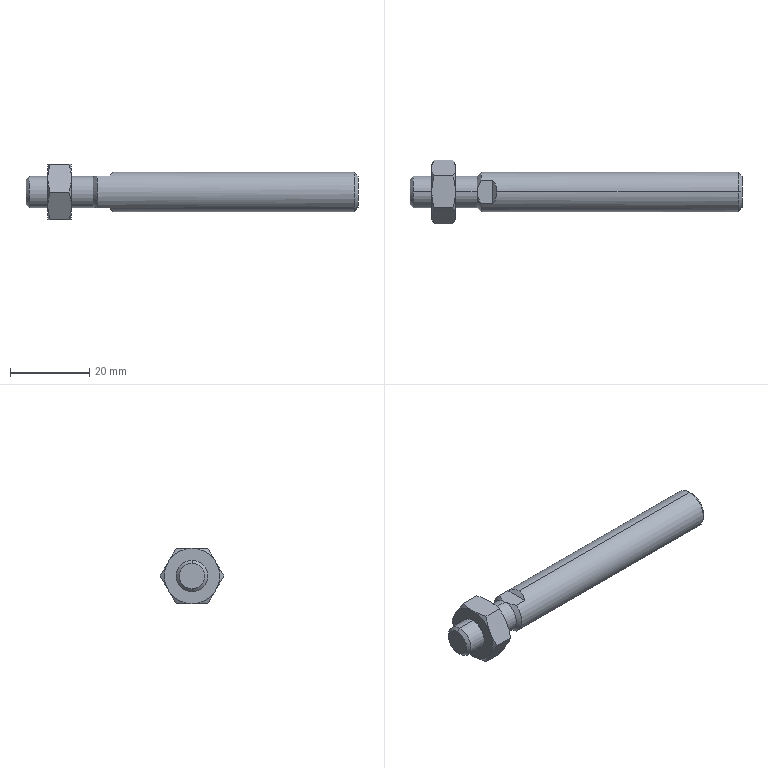Part | SolidWorks | S-SDA25x35-SB(0)_rod.stp | 1 solid | 38 faces | box 84 x 16.166 x 14.001 mm | volume 6760 mm3 | cone 18 | plane 14 | cylinder 6 | commonest cylinder face diameters 8 x4 10 x2
STEP:
#1=CARTESIAN_POINT('',(-16.233,0.,-4.));
#2=VERTEX_POINT('',#1);
#3=CARTESIAN_POINT('',(-16.233,0.,4.));
#4=VERTEX_POINT('',#3);
#5=CARTESIAN_POINT('',(-16.233,0.,0.));
#6=DIRECTION('',(1.,0.,0.));
#7=DIRECTION('',(0.,0.,-1.));
#8=AXIS2_PLACEMENT_3D('',#5,#6,#7);
#9=CIRCLE('',#8,4.);
#10=EDGE_CURVE('',#2,#4,#9,.T.);
#11=ORIENTED_EDGE('',*,*,#10,.T.);
#12=CARTESIAN_POINT('',(-11.5,0.,4.));
#13=VERTEX_POINT('',#12);
#14=CARTESIAN_POINT('',(0.,0.,4.));
#15=DIRECTION('',(1.,0.,0.));
#16=VECTOR('',#15,1000.);
#17=LINE('',#14,#16);
#18=EDGE_CURVE('',#4,#13,#17,.T.);
#19=ORIENTED_EDGE('',*,*,#18,.T.);
#20=CARTESIAN_POINT('',(-11.5,0.,-4.));
#21=VERTEX_POINT('',#20);
#22=CARTESIAN_POINT('',(-11.5,0.,0.));
#23=DIRECTION('',(1.,0.,0.));
#24=DIRECTION('',(0.,0.,-1.));
#25=AXIS2_PLACEMENT_3D('',#22,#23,#24);
#26=CIRCLE('',#25,4.);
#27=EDGE_CURVE('',#21,#13,#26,.T.);
#28=ORIENTED_EDGE('',*,*,#27,.F.);
#29=CARTESIAN_POINT('',(0.,0.,-4.));
#30=DIRECTION('',(1.,0.,0.));
#31=VECTOR('',#30,1000.);
#32=LINE('',#29,#31);
#33=EDGE_CURVE('',#2,#21,#32,.T.);
#34=ORIENTED_EDGE('',*,*,#33,.F.);
#35=EDGE_LOOP('',(#11,#19,#28,#34));
#36=FACE_OUTER_BOUND('',#35,.T.);
#37=CARTESIAN_POINT('',(0.,0.,0.));
#38=DIRECTION('',(1.,0.,0.));
#39=DIRECTION('',(0.,0.,-1.));
#40=AXIS2_PLACEMENT_3D('',#37,#38,#39);
#41=CYLINDRICAL_SURFACE('',#40,4.);
#42=ADVANCED_FACE('',(#36),#41,.T.);
#43=CARTESIAN_POINT('',(-17.,0.,-3.233));
#44=VERTEX_POINT('',#43);
#45=CARTESIAN_POINT('',(-17.,0.,3.233));
#46=VERTEX_POINT('',#45);
#47=CARTESIAN_POINT('',(-17.,0.,0.));
#48=DIRECTION('',(1.,0.,0.));
#49=DIRECTION('',(0.,0.,-1.));
#50=AXIS2_PLACEMENT_3D('',#47,#48,#49);
#51=CIRCLE('',#50,3.233);
#52=EDGE_CURVE('',#44,#46,#51,.T.);
#53=ORIENTED_EDGE('',*,*,#52,.T.);
#54=CARTESIAN_POINT('',(-17.,0.,3.233));
#55=DIRECTION('',(0.7071,0.,0.7071));
#56=VECTOR('',#55,1000.);
#57=LINE('',#54,#56);
#58=EDGE_CURVE('',#46,#4,#57,.T.);
#59=ORIENTED_EDGE('',*,*,#58,.T.);
#60=ORIENTED_EDGE('',*,*,#10,.F.);
#61=CARTESIAN_POINT('',(-17.,0.,-3.233));
#62=DIRECTION('',(0.7071,0.,-0.7071));
#63=VECTOR('',#62,1000.);
#64=LINE('',#61,#63);
#65=EDGE_CURVE('',#44,#2,#64,.T.);
#66=ORIENTED_EDGE('',*,*,#65,.F.);
#67=EDGE_LOOP('',(#53,#59,#60,#66));
#68=FACE_OUTER_BOUND('',#67,.T.);
#69=CARTESIAN_POINT('',(-17.,0.,0.));
#70=DIRECTION('',(1.,0.,0.));
#71=DIRECTION('',(0.,0.,-1.));
#72=AXIS2_PLACEMENT_3D('',#69,#70,#71);
#73=CONICAL_SURFACE('',#72,3.233,0.7854);
#74=ADVANCED_FACE('',(#68),#73,.T.);
#75=CARTESIAN_POINT('',(67.,0.,-4.));
#76=VERTEX_POINT('',#75);
#77=CARTESIAN_POINT('',(67.,0.,4.));
#78=VERTEX_POINT('',#77);
#79=CARTESIAN_POINT('',(67.,0.,0.));
#80=DIRECTION('',(1.,0.,0.));
#81=DIRECTION('',(0.,0.,-1.));
#82=AXIS2_PLACEMENT_3D('',#79,#80,#81);
#83=CIRCLE('',#82,4.);
#84=EDGE_CURVE('',#76,#78,#83,.T.);
#85=ORIENTED_EDGE('',*,*,#84,.F.);
#86=CARTESIAN_POINT('',(66.,0.,-5.));
#87=VERTEX_POINT('',#86);
#88=CARTESIAN_POINT('',(66.,0.,-5.));
#89=DIRECTION('',(-0.7071,0.,-0.7071));
#90=VECTOR('',#89,1000.);
#91=LINE('',#88,#90);
#92=EDGE_CURVE('',#76,#87,#91,.T.);
#93=ORIENTED_EDGE('',*,*,#92,.T.);
#94=CARTESIAN_POINT('',(66.,0.,5.));
#95=VERTEX_POINT('',#94);
#96=CARTESIAN_POINT('',(66.,0.,0.));
#97=DIRECTION('',(1.,0.,0.));
#98=DIRECTION('',(0.,0.,-1.));
#99=AXIS2_PLACEMENT_3D('',#96,#97,#98);
#100=CIRCLE('',#99,5.);
#101=EDGE_CURVE('',#87,#95,#100,.T.);
#102=ORIENTED_EDGE('',*,*,#101,.T.);
#103=CARTESIAN_POINT('',(66.,0.,5.));
#104=DIRECTION('',(-0.7071,0.,0.7071));
#105=VECTOR('',#104,1000.);
#106=LINE('',#103,#105);
#107=EDGE_CURVE('',#78,#95,#106,.T.);
#108=ORIENTED_EDGE('',*,*,#107,.F.);
#109=EDGE_LOOP('',(#85,#93,#102,#108));
#110=FACE_OUTER_BOUND('',#109,.T.);
#111=CARTESIAN_POINT('',(66.,0.,0.));
#112=DIRECTION('',(-1.,0.,0.));
#113=DIRECTION('',(0.,0.,1.));
#114=AXIS2_PLACEMENT_3D('',#111,#112,#113);
#115=CONICAL_SURFACE('',#114,5.,0.7854);
#116=ADVANCED_FACE('',(#110),#115,.T.);
#117=CARTESIAN_POINT('',(5.,0.,5.));
#118=VERTEX_POINT('',#117);
#119=CARTESIAN_POINT('',(4.,3.,4.));
#120=VERTEX_POINT('',#119);
#121=CARTESIAN_POINT('',(5.,0.,5.));
#122=CARTESIAN_POINT('',(5.,1.091,5.));
#123=CARTESIAN_POINT('',(4.655,2.127,4.655));
#124=CARTESIAN_POINT('',(4.,3.,4.));
#125=(BOUNDED_CURVE()B_SPLINE_CURVE(3,(#121,#122,#123,#124),.UNSPECIFIED.,.F.,.F.)B_SPLINE_CURVE_WITH_KNOTS((4,4),(0.,0.6435),.UNSPECIFIED.)CURVE()GEOMETRIC_REPRESENTATION_ITEM()RATIONAL_B_SPLINE_CURVE((1.,0.9658,0.9658,1.))REPRESENTATION_ITEM(''));
#126=EDGE_CURVE('',#118,#120,#125,.T.);
#127=ORIENTED_EDGE('',*,*,#126,.F.);
#128=CARTESIAN_POINT('',(67.,0.,5.));
#129=DIRECTION('',(1.,0.,0.));
#130=VECTOR('',#129,1000.);
#131=LINE('',#128,#130);
#132=EDGE_CURVE('',#118,#95,#131,.T.);
#133=ORIENTED_EDGE('',*,*,#132,.T.);
#134=ORIENTED_EDGE('',*,*,#101,.F.);
#135=CARTESIAN_POINT('',(5.,0.,-5.));
#136=VERTEX_POINT('',#135);
#137=CARTESIAN_POINT('',(67.,0.,-5.));
#138=DIRECTION('',(1.,0.,0.));
#139=VECTOR('',#138,1000.);
#140=LINE('',#137,#139);
#141=EDGE_CURVE('',#136,#87,#140,.T.);
#142=ORIENTED_EDGE('',*,*,#141,.F.);
#143=CARTESIAN_POINT('',(4.,3.,-4.));
#144=VERTEX_POINT('',#143);
#145=CARTESIAN_POINT('',(4.,3.,-4.));
#146=CARTESIAN_POINT('',(4.655,2.127,-4.655));
#147=CARTESIAN_POINT('',(5.,1.091,-5.));
#148=CARTESIAN_POINT('',(5.,0.,-5.));
#149=(BOUNDED_CURVE()B_SPLINE_CURVE(3,(#145,#146,#147,#148),.UNSPECIFIED.,.F.,.F.)B_SPLINE_CURVE_WITH_KNOTS((4,4),(5.64,6.283),.UNSPECIFIED.)CURVE()GEOMETRIC_REPRESENTATION_ITEM()RATIONAL_B_SPLINE_CURVE((1.,0.9658,0.9658,1.))REPRESENTATION_ITEM(''));
#150=EDGE_CURVE('',#144,#136,#149,.T.);
#151=ORIENTED_EDGE('',*,*,#150,.F.);
#152=CARTESIAN_POINT('',(1.,3.,-4.));
#153=VERTEX_POINT('',#152);
#154=CARTESIAN_POINT('',(67.,3.,-4.));
#155=DIRECTION('',(1.,0.,0.));
#156=VECTOR('',#155,1000.);
#157=LINE('',#154,#156);
#158=EDGE_CURVE('',#153,#144,#157,.T.);
#159=ORIENTED_EDGE('',*,*,#158,.F.);
#160=CARTESIAN_POINT('',(1.,3.,4.));
#161=VERTEX_POINT('',#160);
#162=CARTESIAN_POINT('',(1.,0.,0.));
#163=DIRECTION('',(1.,0.,0.));
#164=DIRECTION('',(0.,0.,-1.));
#165=AXIS2_PLACEMENT_3D('',#162,#163,#164);
#166=CIRCLE('',#165,5.);
#167=EDGE_CURVE('',#153,#161,#166,.T.);
#168=ORIENTED_EDGE('',*,*,#167,.T.);
#169=CARTESIAN_POINT('',(67.,3.,4.));
#170=DIRECTION('',(-1.,0.,0.));
#171=VECTOR('',#170,1000.);
#172=LINE('',#169,#171);
#173=EDGE_CURVE('',#120,#161,#172,.T.);
#174=ORIENTED_EDGE('',*,*,#173,.F.);
#175=EDGE_LOOP('',(#127,#133,#134,#142,#151,#159,#168,#174));
#176=FACE_OUTER_BOUND('',#175,.T.);
#177=CARTESIAN_POINT('',(67.,0.,0.));
#178=DIRECTION('',(1.,0.,0.));
#179=DIRECTION('',(0.,0.,-1.));
#180=AXIS2_PLACEMENT_3D('',#177,#178,#179);
#181=CYLINDRICAL_SURFACE('',#180,5.);
#182=ADVANCED_FACE('',(#176),#181,.T.);
#183=CARTESIAN_POINT('',(-5.5,0.,4.));
#184=VERTEX_POINT('',#183);
#185=CARTESIAN_POINT('',(-5.5,0.,-4.));
#186=VERTEX_POINT('',#185);
#187=CARTESIAN_POINT('',(-5.5,0.,0.));
#188=DIRECTION('',(-1.,0.,0.));
#189=DIRECTION('',(0.,0.,1.));
#190=AXIS2_PLACEMENT_3D('',#187,#188,#189);
#191=CIRCLE('',#190,4.);
#192=EDGE_CURVE('',#184,#186,#191,.T.);
#193=ORIENTED_EDGE('',*,*,#192,.F.);
#194=CARTESIAN_POINT('',(0.,0.,4.));
#195=VERTEX_POINT('',#194);
#196=CARTESIAN_POINT('',(0.,0.,4.));
#197=DIRECTION('',(1.,0.,0.));
#198=VECTOR('',#197,1000.);
#199=LINE('',#196,#198);
#200=EDGE_CURVE('',#184,#195,#199,.T.);
#201=ORIENTED_EDGE('',*,*,#200,.T.);
#202=CARTESIAN_POINT('',(0.,0.,-4.));
#203=VERTEX_POINT('',#202);
#204=CARTESIAN_POINT('',(0.,0.,0.));
#205=DIRECTION('',(1.,0.,0.));
#206=DIRECTION('',(0.,0.,-1.));
#207=AXIS2_PLACEMENT_3D('',#204,#205,#206);
#208=CIRCLE('',#207,4.);
#209=EDGE_CURVE('',#203,#195,#208,.T.);
#210=ORIENTED_EDGE('',*,*,#209,.F.);
#211=CARTESIAN_POINT('',(0.,0.,-4.));
#212=DIRECTION('',(1.,0.,0.));
#213=VECTOR('',#212,1000.);
#214=LINE('',#211,#213);
#215=EDGE_CURVE('',#186,#203,#214,.T.);
#216=ORIENTED_EDGE('',*,*,#215,.F.);
#217=EDGE_LOOP('',(#193,#201,#210,#216));
#218=FACE_OUTER_BOUND('',#217,.T.);
#219=CARTESIAN_POINT('',(0.,0.,0.));
#220=DIRECTION('',(1.,0.,0.));
#221=DIRECTION('',(0.,0.,-1.));
#222=AXIS2_PLACEMENT_3D('',#219,#220,#221);
#223=CYLINDRICAL_SURFACE('',#222,4.);
#224=ADVANCED_FACE('',(#218),#223,.T.);
#225=CARTESIAN_POINT('',(-5.5,0.,-7.));
#226=VERTEX_POINT('',#225);
#227=CARTESIAN_POINT('',(-6.125,4.041,-7.));
#228=VERTEX_POINT('',#227);
#229=CARTESIAN_POINT('',(-5.5,0.,-7.));
#230=CARTESIAN_POINT('',(-5.5,0.3423,-7.));
#231=CARTESIAN_POINT('',(-5.514,0.6793,-7.));
#232=CARTESIAN_POINT('',(-5.556,1.187,-7.));
#233=CARTESIAN_POINT('',(-5.574,1.357,-7.));
#234=CARTESIAN_POINT('',(-5.606,1.614,-7.));
#235=CARTESIAN_POINT('',(-5.623,1.742,-7.));
#236=CARTESIAN_POINT('',(-5.645,1.894,-7.));
#237=CARTESIAN_POINT('',(-5.655,1.959,-7.));
#238=CARTESIAN_POINT('',(-5.662,2.002,-7.));
#239=CARTESIAN_POINT('',(-5.666,2.025,-7.));
#240=CARTESIAN_POINT('',(-5.775,2.699,-7.));
#241=CARTESIAN_POINT('',(-5.927,3.355,-7.));
#242=CARTESIAN_POINT('',(-6.125,4.041,-7.));
#243=B_SPLINE_CURVE_WITH_KNOTS('',3,(#229,#230,#231,#232,#233,#234,#235,#236,#237,#238,#239,#240,#241,#242),.UNSPECIFIED.,.F.,.F.,(4,2,2,1,1,2,2,4),(0.,0.25,0.375,0.4375,0.4687,0.4844,0.5,1.),.UNSPECIFIED.);
#244=EDGE_CURVE('',#226,#228,#243,.T.);
#245=ORIENTED_EDGE('',*,*,#244,.T.);
#246=CARTESIAN_POINT('',(-5.5,6.062,-3.5));
#247=VERTEX_POINT('',#246);
#248=CARTESIAN_POINT('',(-6.125,4.041,-7.));
#249=CARTESIAN_POINT('',(-6.026,4.213,-6.702));
#250=CARTESIAN_POINT('',(-5.938,4.382,-6.411));
#251=CARTESIAN_POINT('',(-5.824,4.631,-5.979));
#252=CARTESIAN_POINT('',(-5.789,4.714,-5.836));
#253=CARTESIAN_POINT('',(-5.741,4.837,-5.623));
#254=CARTESIAN_POINT('',(-5.717,4.899,-5.516));
#255=CARTESIAN_POINT('',(-5.692,4.97,-5.392));
#256=CARTESIAN_POINT('',(-5.682,5.001,-5.339));
#257=CARTESIAN_POINT('',(-5.675,5.021,-5.304));
#258=CARTESIAN_POINT('',(-5.672,5.031,-5.287));
#259=CARTESIAN_POINT('',(-5.556,5.39,-4.666));
#260=CARTESIAN_POINT('',(-5.5,5.721,-4.091));
#261=CARTESIAN_POINT('',(-5.5,6.062,-3.5));
#262=B_SPLINE_CURVE_WITH_KNOTS('',3,(#248,#249,#250,#251,#252,#253,#254,#255,#256,#257,#258,#259,#260,#261),.UNSPECIFIED.,.F.,.F.,(4,2,2,1,1,2,2,4),(0.,0.25,0.375,0.4375,0.4688,0.4844,0.5,1.),.UNSPECIFIED.);
#263=EDGE_CURVE('',#228,#247,#262,.T.);
#264=ORIENTED_EDGE('',*,*,#263,.T.);
#265=CARTESIAN_POINT('',(-5.5,0.,0.));
#266=DIRECTION('',(1.,0.,0.));
#267=DIRECTION('',(0.,0.,-1.));
#268=AXIS2_PLACEMENT_3D('',#265,#266,#267);
#269=CIRCLE('',#268,7.);
#270=EDGE_CURVE('',#226,#247,#269,.T.);
#271=ORIENTED_EDGE('',*,*,#270,.F.);
#272=EDGE_LOOP('',(#245,#264,#271));
#273=FACE_OUTER_BOUND('',#272,.T.);
#274=CARTESIAN_POINT('',(-8.5,0.,0.));
#275=DIRECTION('',(-1.,0.,0.));
#276=DIRECTION('',(0.,0.,1.));
#277=AXIS2_PLACEMENT_3D('',#274,#275,#276);
#278=CONICAL_SURFACE('',#277,12.196,1.047);
#279=ADVANCED_FACE('',(#273),#278,.T.);
#280=CARTESIAN_POINT('',(-5.5,6.062,3.5));
#281=VERTEX_POINT('',#280);
#282=CARTESIAN_POINT('',(-5.5,0.,0.));
#283=DIRECTION('',(1.,0.,0.));
#284=DIRECTION('',(0.,0.,-1.));
#285=AXIS2_PLACEMENT_3D('',#282,#283,#284);
#286=CIRCLE('',#285,7.);
#287=EDGE_CURVE('',#247,#281,#286,.T.);
#288=ORIENTED_EDGE('',*,*,#287,.F.);
#289=CARTESIAN_POINT('',(-6.125,8.083,0.));
#290=VERTEX_POINT('',#289);
#291=CARTESIAN_POINT('',(-5.5,6.062,-3.5));
#292=CARTESIAN_POINT('',(-5.5,6.233,-3.205));
#293=CARTESIAN_POINT('',(-5.514,6.4,-2.913));
#294=CARTESIAN_POINT('',(-5.556,6.654,-2.475));
#295=CARTESIAN_POINT('',(-5.574,6.739,-2.328));
#296=CARTESIAN_POINT('',(-5.605,6.867,-2.106));
#297=CARTESIAN_POINT('',(-5.623,6.932,-1.995));
#298=CARTESIAN_POINT('',(-5.645,7.007,-1.864));
#299=CARTESIAN_POINT('',(-5.655,7.04,-1.808));
#300=CARTESIAN_POINT('',(-5.662,7.061,-1.771));
#301=CARTESIAN_POINT('',(-5.665,7.073,-1.751));
#302=CARTESIAN_POINT('',(-5.774,7.411,-1.166));
#303=CARTESIAN_POINT('',(-5.927,7.739,-0.5958));
#304=CARTESIAN_POINT('',(-6.125,8.083,0.));
#305=B_SPLINE_CURVE_WITH_KNOTS('',3,(#291,#292,#293,#294,#295,#296,#297,#298,#299,#300,#301,#302,#303,#304),.UNSPECIFIED.,.F.,.F.,(4,2,2,1,1,2,2,4),(0.,0.25,0.375,0.4375,0.4688,0.4844,0.5,1.),.UNSPECIFIED.);
#306=EDGE_CURVE('',#247,#290,#305,.T.);
#307=ORIENTED_EDGE('',*,*,#306,.T.);
#308=CARTESIAN_POINT('',(-6.125,8.083,0.));
#309=CARTESIAN_POINT('',(-6.026,7.911,0.298));
#310=CARTESIAN_POINT('',(-5.938,7.743,0.5894));
#311=CARTESIAN_POINT('',(-5.824,7.494,1.021));
#312=CARTESIAN_POINT('',(-5.789,7.411,1.164));
#313=CARTESIAN_POINT('',(-5.741,7.288,1.378));
#314=CARTESIAN_POINT('',(-5.717,7.226,1.484));
#315=CARTESIAN_POINT('',(-5.692,7.155,1.608));
#316=CARTESIAN_POINT('',(-5.682,7.124,1.661));
#317=CARTESIAN_POINT('',(-5.675,7.104,1.697));
#318=CARTESIAN_POINT('',(-5.672,7.094,1.713));
#319=CARTESIAN_POINT('',(-5.556,6.735,2.335));
#320=CARTESIAN_POINT('',(-5.5,6.404,2.909));
#321=CARTESIAN_POINT('',(-5.5,6.062,3.5));
#322=B_SPLINE_CURVE_WITH_KNOTS('',3,(#308,#309,#310,#311,#312,#313,#314,#315,#316,#317,#318,#319,#320,#321),.UNSPECIFIED.,.F.,.F.,(4,2,2,1,1,2,2,4),(0.,0.25,0.375,0.4375,0.4688,0.4844,0.5,1.),.UNSPECIFIED.);
#323=EDGE_CURVE('',#290,#281,#322,.T.);
#324=ORIENTED_EDGE('',*,*,#323,.T.);
#325=EDGE_LOOP('',(#288,#307,#324));
#326=FACE_OUTER_BOUND('',#325,.T.);
#327=CARTESIAN_POINT('',(-8.5,0.,0.));
#328=DIRECTION('',(-1.,0.,0.));
#329=DIRECTION('',(0.,0.,1.));
#330=AXIS2_PLACEMENT_3D('',#327,#328,#329);
#331=CONICAL_SURFACE('',#330,12.196,1.047);
#332=ADVANCED_FACE('',(#326),#331,.T.);
#333=CARTESIAN_POINT('',(-5.5,0.,7.));
#334=VERTEX_POINT('',#333);
#335=CARTESIAN_POINT('',(-5.5,0.,0.));
#336=DIRECTION('',(1.,0.,0.));
#337=DIRECTION('',(0.,0.,-1.));
#338=AXIS2_PLACEMENT_3D('',#335,#336,#337);
#339=CIRCLE('',#338,7.);
#340=EDGE_CURVE('',#281,#334,#339,.T.);
#341=ORIENTED_EDGE('',*,*,#340,.F.);
#342=CARTESIAN_POINT('',(-6.125,4.041,7.));
#343=VERTEX_POINT('',#342);
#344=CARTESIAN_POINT('',(-5.5,6.062,3.5));
#345=CARTESIAN_POINT('',(-5.5,5.892,3.795));
#346=CARTESIAN_POINT('',(-5.514,5.723,4.086));
#347=CARTESIAN_POINT('',(-5.556,5.47,4.525));
#348=CARTESIAN_POINT('',(-5.574,5.386,4.672));
#349=CARTESIAN_POINT('',(-5.605,5.258,4.894));
#350=CARTESIAN_POINT('',(-5.623,5.194,5.005));
#351=CARTESIAN_POINT('',(-5.645,5.118,5.136));
#352=CARTESIAN_POINT('',(-5.655,5.086,5.192));
#353=CARTESIAN_POINT('',(-5.662,5.064,5.23));
#354=CARTESIAN_POINT('',(-5.665,5.053,5.25));
#355=CARTESIAN_POINT('',(-5.774,4.715,5.835));
#356=CARTESIAN_POINT('',(-5.927,4.385,6.404));
#357=CARTESIAN_POINT('',(-6.125,4.041,7.));
#358=B_SPLINE_CURVE_WITH_KNOTS('',3,(#344,#345,#346,#347,#348,#349,#350,#351,#352,#353,#354,#355,#356,#357),.UNSPECIFIED.,.F.,.F.,(4,2,2,1,1,2,2,4),(0.,0.25,0.375,0.4375,0.4688,0.4844,0.5,1.),.UNSPECIFIED.);
#359=EDGE_CURVE('',#281,#343,#358,.T.);
#360=ORIENTED_EDGE('',*,*,#359,.T.);
#361=CARTESIAN_POINT('',(-6.125,4.041,7.));
#362=CARTESIAN_POINT('',(-6.026,3.698,7.));
#363=CARTESIAN_POINT('',(-5.939,3.363,7.));
#364=CARTESIAN_POINT('',(-5.825,2.865,7.));
#365=CARTESIAN_POINT('',(-5.79,2.701,7.));
#366=CARTESIAN_POINT('',(-5.741,2.455,7.));
#367=CARTESIAN_POINT('',(-5.718,2.332,7.));
#368=CARTESIAN_POINT('',(-5.693,2.189,7.));
#369=CARTESIAN_POINT('',(-5.683,2.128,7.001));
#370=CARTESIAN_POINT('',(-5.676,2.087,7.001));
#371=CARTESIAN_POINT('',(-5.673,2.068,7.001));
#372=CARTESIAN_POINT('',(-5.556,1.349,7.001));
#373=CARTESIAN_POINT('',(-5.5,0.6844,7.));
#374=CARTESIAN_POINT('',(-5.5,0.,7.));
#375=B_SPLINE_CURVE_WITH_KNOTS('',3,(#361,#362,#363,#364,#365,#366,#367,#368,#369,#370,#371,#372,#373,#374),.UNSPECIFIED.,.F.,.F.,(4,2,2,1,1,2,2,4),(0.,0.25,0.375,0.4375,0.4687,0.4844,0.5,1.),.UNSPECIFIED.);
#376=EDGE_CURVE('',#343,#334,#375,.T.);
#377=ORIENTED_EDGE('',*,*,#376,.T.);
#378=EDGE_LOOP('',(#341,#360,#377));
#379=FACE_OUTER_BOUND('',#378,.T.);
#380=CARTESIAN_POINT('',(-8.5,0.,0.));
#381=DIRECTION('',(-1.,0.,0.));
#382=DIRECTION('',(0.,0.,1.));
#383=AXIS2_PLACEMENT_3D('',#380,#381,#382);
#384=CONICAL_SURFACE('',#383,12.196,1.047);
#385=ADVANCED_FACE('',(#379),#384,.T.);
#386=CARTESIAN_POINT('',(-5.5,-6.062,-3.5));
#387=VERTEX_POINT('',#386);
#388=CARTESIAN_POINT('',(-6.125,-4.041,-7.));
#389=VERTEX_POINT('',#388);
#390=CARTESIAN_POINT('',(-5.5,-6.062,-3.5));
#391=CARTESIAN_POINT('',(-5.5,-5.892,-3.795));
#392=CARTESIAN_POINT('',(-5.514,-5.723,-4.086));
#393=CARTESIAN_POINT('',(-5.556,-5.47,-4.525));
#394=CARTESIAN_POINT('',(-5.574,-5.386,-4.672));
#395=CARTESIAN_POINT('',(-5.605,-5.258,-4.894));
#396=CARTESIAN_POINT('',(-5.623,-5.194,-5.005));
#397=CARTESIAN_POINT('',(-5.645,-5.118,-5.136));
#398=CARTESIAN_POINT('',(-5.655,-5.086,-5.192));
#399=CARTESIAN_POINT('',(-5.662,-5.064,-5.23));
#400=CARTESIAN_POINT('',(-5.665,-5.053,-5.25));
#401=CARTESIAN_POINT('',(-5.774,-4.715,-5.835));
#402=CARTESIAN_POINT('',(-5.927,-4.385,-6.404));
#403=CARTESIAN_POINT('',(-6.125,-4.041,-7.));
#404=B_SPLINE_CURVE_WITH_KNOTS('',3,(#390,#391,#392,#393,#394,#395,#396,#397,#398,#399,#400,#401,#402,#403),.UNSPECIFIED.,.F.,.F.,(4,2,2,1,1,2,2,4),(0.,0.25,0.375,0.4375,0.4687,0.4844,0.5,1.),.UNSPECIFIED.);
#405=EDGE_CURVE('',#387,#389,#404,.T.);
#406=ORIENTED_EDGE('',*,*,#405,.T.);
#407=CARTESIAN_POINT('',(-6.125,-4.041,-7.));
#408=CARTESIAN_POINT('',(-6.026,-3.698,-7.));
#409=CARTESIAN_POINT('',(-5.939,-3.363,-7.));
#410=CARTESIAN_POINT('',(-5.825,-2.865,-7.));
#411=CARTESIAN_POINT('',(-5.79,-2.701,-7.));
#412=CARTESIAN_POINT('',(-5.741,-2.455,-7.));
#413=CARTESIAN_POINT('',(-5.718,-2.332,-7.));
#414=CARTESIAN_POINT('',(-5.693,-2.189,-7.));
#415=CARTESIAN_POINT('',(-5.683,-2.128,-7.001));
#416=CARTESIAN_POINT('',(-5.676,-2.087,-7.001));
#417=CARTESIAN_POINT('',(-5.673,-2.068,-7.001));
#418=CARTESIAN_POINT('',(-5.556,-1.349,-7.001));
#419=CARTESIAN_POINT('',(-5.5,-0.6844,-7.));
#420=CARTESIAN_POINT('',(-5.5,0.,-7.));
#421=B_SPLINE_CURVE_WITH_KNOTS('',3,(#407,#408,#409,#410,#411,#412,#413,#414,#415,#416,#417,#418,#419,#420),.UNSPECIFIED.,.F.,.F.,(4,2,2,1,1,2,2,4),(0.,0.25,0.375,0.4375,0.4688,0.4844,0.5,1.),.UNSPECIFIED.);
#422=EDGE_CURVE('',#389,#226,#421,.T.);
#423=ORIENTED_EDGE('',*,*,#422,.T.);
#424=CARTESIAN_POINT('',(-5.5,0.,0.));
#425=DIRECTION('',(1.,0.,0.));
#426=DIRECTION('',(0.,0.,-1.));
#427=AXIS2_PLACEMENT_3D('',#424,#425,#426);
#428=CIRCLE('',#427,7.);
#429=EDGE_CURVE('',#387,#226,#428,.T.);
#430=ORIENTED_EDGE('',*,*,#429,.F.);
#431=EDGE_LOOP('',(#406,#423,#430));
#432=FACE_OUTER_BOUND('',#431,.T.);
#433=CARTESIAN_POINT('',(-8.5,0.,0.));
#434=DIRECTION('',(-1.,0.,0.));
#435=DIRECTION('',(0.,0.,1.));
#436=AXIS2_PLACEMENT_3D('',#433,#434,#435);
#437=CONICAL_SURFACE('',#436,12.196,1.047);
#438=ADVANCED_FACE('',(#432),#437,.T.);
#439=CARTESIAN_POINT('',(-5.5,-6.062,3.5));
#440=VERTEX_POINT('',#439);
#441=CARTESIAN_POINT('',(-5.5,0.,0.));
#442=DIRECTION('',(1.,0.,0.));
#443=DIRECTION('',(0.,0.,-1.));
#444=AXIS2_PLACEMENT_3D('',#441,#442,#443);
#445=CIRCLE('',#444,7.);
#446=EDGE_CURVE('',#334,#440,#445,.T.);
#447=ORIENTED_EDGE('',*,*,#446,.F.);
#448=CARTESIAN_POINT('',(-6.125,-4.041,7.));
#449=VERTEX_POINT('',#448);
#450=CARTESIAN_POINT('',(-5.5,0.,7.));
#451=CARTESIAN_POINT('',(-5.5,-0.3423,7.));
#452=CARTESIAN_POINT('',(-5.514,-0.6793,7.));
#453=CARTESIAN_POINT('',(-5.556,-1.187,7.));
#454=CARTESIAN_POINT('',(-5.574,-1.357,7.));
#455=CARTESIAN_POINT('',(-5.606,-1.614,7.));
#456=CARTESIAN_POINT('',(-5.623,-1.742,7.));
#457=CARTESIAN_POINT('',(-5.645,-1.894,7.));
#458=CARTESIAN_POINT('',(-5.655,-1.959,7.));
#459=CARTESIAN_POINT('',(-5.662,-2.002,7.));
#460=CARTESIAN_POINT('',(-5.666,-2.025,7.));
#461=CARTESIAN_POINT('',(-5.775,-2.699,7.));
#462=CARTESIAN_POINT('',(-5.927,-3.355,7.));
#463=CARTESIAN_POINT('',(-6.125,-4.041,7.));
#464=B_SPLINE_CURVE_WITH_KNOTS('',3,(#450,#451,#452,#453,#454,#455,#456,#457,#458,#459,#460,#461,#462,#463),.UNSPECIFIED.,.F.,.F.,(4,2,2,1,1,2,2,4),(0.,0.25,0.375,0.4375,0.4688,0.4844,0.5,1.),.UNSPECIFIED.);
#465=EDGE_CURVE('',#334,#449,#464,.T.);
#466=ORIENTED_EDGE('',*,*,#465,.T.);
#467=CARTESIAN_POINT('',(-6.125,-4.041,7.));
#468=CARTESIAN_POINT('',(-6.026,-4.213,6.702));
#469=CARTESIAN_POINT('',(-5.938,-4.382,6.411));
#470=CARTESIAN_POINT('',(-5.824,-4.631,5.979));
#471=CARTESIAN_POINT('',(-5.789,-4.714,5.836));
#472=CARTESIAN_POINT('',(-5.741,-4.837,5.623));
#473=CARTESIAN_POINT('',(-5.717,-4.899,5.516));
#474=CARTESIAN_POINT('',(-5.692,-4.97,5.392));
#475=CARTESIAN_POINT('',(-5.682,-5.001,5.339));
#476=CARTESIAN_POINT('',(-5.675,-5.021,5.304));
#477=CARTESIAN_POINT('',(-5.672,-5.031,5.287));
#478=CARTESIAN_POINT('',(-5.556,-5.39,4.666));
#479=CARTESIAN_POINT('',(-5.5,-5.721,4.091));
#480=CARTESIAN_POINT('',(-5.5,-6.062,3.5));
#481=B_SPLINE_CURVE_WITH_KNOTS('',3,(#467,#468,#469,#470,#471,#472,#473,#474,#475,#476,#477,#478,#479,#480),.UNSPECIFIED.,.F.,.F.,(4,2,2,1,1,2,2,4),(0.,0.25,0.375,0.4375,0.4688,0.4844,0.5,1.),.UNSPECIFIED.);
#482=EDGE_CURVE('',#449,#440,#481,.T.);
#483=ORIENTED_EDGE('',*,*,#482,.T.);
#484=EDGE_LOOP('',(#447,#466,#483));
#485=FACE_OUTER_BOUND('',#484,.T.);
#486=CARTESIAN_POINT('',(-8.5,0.,0.));
#487=DIRECTION('',(-1.,0.,0.));
#488=DIRECTION('',(0.,0.,1.));
#489=AXIS2_PLACEMENT_3D('',#486,#487,#488);
#490=CONICAL_SURFACE('',#489,12.196,1.047);
#491=ADVANCED_FACE('',(#485),#490,.T.);
#492=ORIENTED_EDGE('',*,*,#200,.F.);
#493=CARTESIAN_POINT('',(-5.5,0.,0.));
#494=DIRECTION('',(-1.,0.,0.));
#495=DIRECTION('',(0.,0.,1.));
#496=AXIS2_PLACEMENT_3D('',#493,#494,#495);
#497=CIRCLE('',#496,4.);
#498=EDGE_CURVE('',#186,#184,#497,.T.);
#499=ORIENTED_EDGE('',*,*,#498,.F.);
#500=ORIENTED_EDGE('',*,*,#215,.T.);
#501=CARTESIAN_POINT('',(0.,0.,0.));
#502=DIRECTION('',(1.,0.,0.));
#503=DIRECTION('',(0.,0.,-1.));
#504=AXIS2_PLACEMENT_3D('',#501,#502,#503);
#505=CIRCLE('',#504,4.);
#506=EDGE_CURVE('',#195,#203,#505,.T.);
#507=ORIENTED_EDGE('',*,*,#506,.F.);
#508=EDGE_LOOP('',(#492,#499,#500,#507));
#509=FACE_OUTER_BOUND('',#508,.T.);
#510=CARTESIAN_POINT('',(0.,0.,0.));
#511=DIRECTION('',(1.,0.,0.));
#512=DIRECTION('',(0.,0.,-1.));
#513=AXIS2_PLACEMENT_3D('',#510,#511,#512);
#514=CYLINDRICAL_SURFACE('',#513,4.);
#515=ADVANCED_FACE('',(#509),#514,.T.);
#516=CARTESIAN_POINT('',(1.,3.,4.));
#517=CARTESIAN_POINT('',(0.8443,2.741,4.));
#518=CARTESIAN_POINT('',(0.6399,2.368,4.));
#519=CARTESIAN_POINT('',(0.4523,1.961,4.));
#520=CARTESIAN_POINT('',(0.3712,1.765,4.));
#521=CARTESIAN_POINT('',(0.3339,1.669,4.));
#522=CARTESIAN_POINT('',(0.316,1.622,4.));
#523=CARTESIAN_POINT('',(0.3085,1.601,4.));
#524=CARTESIAN_POINT('',(0.3035,1.588,4.));
#525=CARTESIAN_POINT('',(0.3017,1.583,4.));
#526=CARTESIAN_POINT('',(0.09954,1.024,4.));
#527=CARTESIAN_POINT('',(0.,0.4995,4.));
#528=CARTESIAN_POINT('',(0.,0.,4.));
#529=B_SPLINE_CURVE_WITH_KNOTS('',3,(#516,#517,#518,#519,#520,#521,#522,#523,#524,#525,#526,#527,#528),.UNSPECIFIED.,.F.,.F.,(4,1,1,1,1,1,2,2,4),(0.,0.25,0.375,0.4375,0.4688,0.4844,0.4922,0.5,1.),.UNSPECIFIED.);
#530=EDGE_CURVE('',#161,#195,#529,.T.);
#531=ORIENTED_EDGE('',*,*,#530,.F.);
#532=ORIENTED_EDGE('',*,*,#167,.F.);
#533=CARTESIAN_POINT('',(0.,0.,-4.));
#534=CARTESIAN_POINT('',(0.,0.249,-4.));
#535=CARTESIAN_POINT('',(0.03698,0.6316,-4.));
#536=CARTESIAN_POINT('',(0.1448,1.094,-4.));
#537=CARTESIAN_POINT('',(0.215,1.329,-4.));
#538=CARTESIAN_POINT('',(0.2541,1.447,-4.));
#539=CARTESIAN_POINT('',(0.2746,1.507,-4.));
#540=CARTESIAN_POINT('',(0.2836,1.533,-4.));
#541=CARTESIAN_POINT('',(0.2897,1.55,-4.));
#542=CARTESIAN_POINT('',(0.2934,1.56,-4.));
#543=CARTESIAN_POINT('',(0.4528,2.001,-4.));
#544=CARTESIAN_POINT('',(0.6875,2.479,-4.));
#545=CARTESIAN_POINT('',(1.,3.,-4.));
#546=B_SPLINE_CURVE_WITH_KNOTS('',3,(#533,#534,#535,#536,#537,#538,#539,#540,#541,#542,#543,#544,#545),.UNSPECIFIED.,.F.,.F.,(4,1,1,1,1,1,2,2,4),(0.,0.25,0.375,0.4375,0.4688,0.4844,0.4922,0.5,1.),.UNSPECIFIED.);
#547=EDGE_CURVE('',#203,#153,#546,.T.);
#548=ORIENTED_EDGE('',*,*,#547,.F.);
#549=ORIENTED_EDGE('',*,*,#209,.T.);
#550=EDGE_LOOP('',(#531,#532,#548,#549));
#551=FACE_OUTER_BOUND('',#550,.T.);
#552=CARTESIAN_POINT('',(0.,0.,0.));
#553=DIRECTION('',(1.,0.,0.));
#554=DIRECTION('',(0.,0.,-1.));
#555=AXIS2_PLACEMENT_3D('',#552,#553,#554);
#556=CONICAL_SURFACE('',#555,4.,0.7854);
#557=ADVANCED_FACE('',(#551),#556,.T.);
#558=CARTESIAN_POINT('',(1.,-3.,4.));
#559=VERTEX_POINT('',#558);
#560=CARTESIAN_POINT('',(0.,0.,4.));
#561=CARTESIAN_POINT('',(0.,-0.249,4.));
#562=CARTESIAN_POINT('',(0.03698,-0.6316,4.));
#563=CARTESIAN_POINT('',(0.1448,-1.094,4.));
#564=CARTESIAN_POINT('',(0.215,-1.329,4.));
#565=CARTESIAN_POINT('',(0.2541,-1.447,4.));
#566=CARTESIAN_POINT('',(0.2746,-1.507,4.));
#567=CARTESIAN_POINT('',(0.2836,-1.533,4.));
#568=CARTESIAN_POINT('',(0.2897,-1.55,4.));
#569=CARTESIAN_POINT('',(0.2934,-1.56,4.));
#570=CARTESIAN_POINT('',(0.4528,-2.001,4.));
#571=CARTESIAN_POINT('',(0.6875,-2.479,4.));
#572=CARTESIAN_POINT('',(1.,-3.,4.));
#573=B_SPLINE_CURVE_WITH_KNOTS('',3,(#560,#561,#562,#563,#564,#565,#566,#567,#568,#569,#570,#571,#572),.UNSPECIFIED.,.F.,.F.,(4,1,1,1,1,1,2,2,4),(0.,0.25,0.375,0.4375,0.4688,0.4844,0.4922,0.5,1.),.UNSPECIFIED.);
#574=EDGE_CURVE('',#195,#559,#573,.T.);
#575=ORIENTED_EDGE('',*,*,#574,.F.);
#576=ORIENTED_EDGE('',*,*,#506,.T.);
#577=CARTESIAN_POINT('',(1.,-3.,-4.));
#578=VERTEX_POINT('',#577);
#579=CARTESIAN_POINT('',(1.,-3.,-4.));
#580=CARTESIAN_POINT('',(0.8443,-2.741,-4.));
#581=CARTESIAN_POINT('',(0.6399,-2.368,-4.));
#582=CARTESIAN_POINT('',(0.4523,-1.961,-4.));
#583=CARTESIAN_POINT('',(0.3712,-1.765,-4.));
#584=CARTESIAN_POINT('',(0.3339,-1.669,-4.));
#585=CARTESIAN_POINT('',(0.316,-1.622,-4.));
#586=CARTESIAN_POINT('',(0.3085,-1.601,-4.));
#587=CARTESIAN_POINT('',(0.3035,-1.588,-4.));
#588=CARTESIAN_POINT('',(0.3017,-1.583,-4.));
#589=CARTESIAN_POINT('',(0.09954,-1.024,-4.));
#590=CARTESIAN_POINT('',(0.,-0.4995,-4.));
#591=CARTESIAN_POINT('',(0.,0.,-4.));
#592=B_SPLINE_CURVE_WITH_KNOTS('',3,(#579,#580,#581,#582,#583,#584,#585,#586,#587,#588,#589,#590,#591),.UNSPECIFIED.,.F.,.F.,(4,1,1,1,1,1,2,2,4),(0.,0.25,0.375,0.4375,0.4688,0.4844,0.4922,0.5,1.),.UNSPECIFIED.);
#593=EDGE_CURVE('',#578,#203,#592,.T.);
#594=ORIENTED_EDGE('',*,*,#593,.F.);
#595=CARTESIAN_POINT('',(1.,0.,0.));
#596=DIRECTION('',(1.,0.,0.));
#597=DIRECTION('',(0.,0.,-1.));
#598=AXIS2_PLACEMENT_3D('',#595,#596,#597);
#599=CIRCLE('',#598,5.);
#600=EDGE_CURVE('',#559,#578,#599,.T.);
#601=ORIENTED_EDGE('',*,*,#600,.F.);
#602=EDGE_LOOP('',(#575,#576,#594,#601));
#603=FACE_OUTER_BOUND('',#602,.T.);
#604=CARTESIAN_POINT('',(0.,0.,0.));
#605=DIRECTION('',(1.,0.,0.));
#606=DIRECTION('',(0.,0.,-1.));
#607=AXIS2_PLACEMENT_3D('',#604,#605,#606);
#608=CONICAL_SURFACE('',#607,4.,0.7854);
#609=ADVANCED_FACE('',(#603),#608,.T.);
#610=ORIENTED_EDGE('',*,*,#132,.F.);
#611=CARTESIAN_POINT('',(4.,-3.,4.));
#612=VERTEX_POINT('',#611);
#613=CARTESIAN_POINT('',(4.,-3.,4.));
#614=CARTESIAN_POINT('',(4.655,-2.127,4.655));
#615=CARTESIAN_POINT('',(5.,-1.091,5.));
#616=CARTESIAN_POINT('',(5.,0.,5.));
#617=(BOUNDED_CURVE()B_SPLINE_CURVE(3,(#613,#614,#615,#616),.UNSPECIFIED.,.F.,.F.)B_SPLINE_CURVE_WITH_KNOTS((4,4),(5.64,6.283),.UNSPECIFIED.)CURVE()GEOMETRIC_REPRESENTATION_ITEM()RATIONAL_B_SPLINE_CURVE((1.,0.9658,0.9658,1.))REPRESENTATION_ITEM(''));
#618=EDGE_CURVE('',#612,#118,#617,.T.);
#619=ORIENTED_EDGE('',*,*,#618,.F.);
#620=CARTESIAN_POINT('',(67.,-3.,4.));
#621=DIRECTION('',(1.,0.,0.));
#622=VECTOR('',#621,1000.);
#623=LINE('',#620,#622);
#624=EDGE_CURVE('',#559,#612,#623,.T.);
#625=ORIENTED_EDGE('',*,*,#624,.F.);
#626=ORIENTED_EDGE('',*,*,#600,.T.);
#627=CARTESIAN_POINT('',(4.,-3.,-4.));
#628=VERTEX_POINT('',#627);
#629=CARTESIAN_POINT('',(67.,-3.,-4.));
#630=DIRECTION('',(-1.,0.,0.));
#631=VECTOR('',#630,1000.);
#632=LINE('',#629,#631);
#633=EDGE_CURVE('',#628,#578,#632,.T.);
#634=ORIENTED_EDGE('',*,*,#633,.F.);
#635=CARTESIAN_POINT('',(5.,0.,-5.));
#636=CARTESIAN_POINT('',(5.,-1.091,-5.));
#637=CARTESIAN_POINT('',(4.655,-2.127,-4.655));
#638=CARTESIAN_POINT('',(4.,-3.,-4.));
#639=(BOUNDED_CURVE()B_SPLINE_CURVE(3,(#635,#636,#637,#638),.UNSPECIFIED.,.F.,.F.)B_SPLINE_CURVE_WITH_KNOTS((4,4),(0.,0.6435),.UNSPECIFIED.)CURVE()GEOMETRIC_REPRESENTATION_ITEM()RATIONAL_B_SPLINE_CURVE((1.,0.9658,0.9658,1.))REPRESENTATION_ITEM(''));
#640=EDGE_CURVE('',#136,#628,#639,.T.);
#641=ORIENTED_EDGE('',*,*,#640,.F.);
#642=ORIENTED_EDGE('',*,*,#141,.T.);
#643=CARTESIAN_POINT('',(66.,0.,0.));
#644=DIRECTION('',(1.,0.,0.));
#645=DIRECTION('',(0.,0.,-1.));
#646=AXIS2_PLACEMENT_3D('',#643,#644,#645);
#647=CIRCLE('',#646,5.);
#648=EDGE_CURVE('',#95,#87,#647,.T.);
#649=ORIENTED_EDGE('',*,*,#648,.F.);
#650=EDGE_LOOP('',(#610,#619,#625,#626,#634,#641,#642,#649));
#651=FACE_OUTER_BOUND('',#650,.T.);
#652=CARTESIAN_POINT('',(67.,0.,0.));
#653=DIRECTION('',(1.,0.,0.));
#654=DIRECTION('',(0.,0.,-1.));
#655=AXIS2_PLACEMENT_3D('',#652,#653,#654);
#656=CYLINDRICAL_SURFACE('',#655,5.);
#657=ADVANCED_FACE('',(#651),#656,.T.);
#658=ORIENTED_EDGE('',*,*,#92,.F.);
#659=CARTESIAN_POINT('',(67.,0.,0.));
#660=DIRECTION('',(1.,0.,0.));
#661=DIRECTION('',(0.,0.,-1.));
#662=AXIS2_PLACEMENT_3D('',#659,#660,#661);
#663=CIRCLE('',#662,4.);
#664=EDGE_CURVE('',#78,#76,#663,.T.);
#665=ORIENTED_EDGE('',*,*,#664,.F.);
#666=ORIENTED_EDGE('',*,*,#107,.T.);
#667=ORIENTED_EDGE('',*,*,#648,.T.);
#668=EDGE_LOOP('',(#658,#665,#666,#667));
#669=FACE_OUTER_BOUND('',#668,.T.);
#670=CARTESIAN_POINT('',(66.,0.,0.));
#671=DIRECTION('',(-1.,0.,0.));
#672=DIRECTION('',(0.,0.,1.));
#673=AXIS2_PLACEMENT_3D('',#670,#671,#672);
#674=CONICAL_SURFACE('',#673,5.,0.7854);
#675=ADVANCED_FACE('',(#669),#674,.T.);
#676=ORIENTED_EDGE('',*,*,#664,.T.);
#677=ORIENTED_EDGE('',*,*,#84,.T.);
#678=EDGE_LOOP('',(#676,#677));
#679=FACE_OUTER_BOUND('',#678,.T.);
#680=CARTESIAN_POINT('',(67.,4.,0.));
#681=DIRECTION('',(-1.,0.,0.));
#682=DIRECTION('',(0.,0.,1.));
#683=AXIS2_PLACEMENT_3D('',#680,#681,#682);
#684=PLANE('',#683);
#685=ADVANCED_FACE('',(#679),#684,.F.);
#686=ORIENTED_EDGE('',*,*,#150,.T.);
#687=ORIENTED_EDGE('',*,*,#640,.T.);
#688=CARTESIAN_POINT('',(4.,10.,-4.));
#689=DIRECTION('',(0.,-1.,0.));
#690=VECTOR('',#689,1000.);
#691=LINE('',#688,#690);
#692=EDGE_CURVE('',#144,#628,#691,.T.);
#693=ORIENTED_EDGE('',*,*,#692,.F.);
#694=EDGE_LOOP('',(#686,#687,#693));
#695=FACE_OUTER_BOUND('',#694,.T.);
#696=CARTESIAN_POINT('',(4.,10.,-4.));
#697=DIRECTION('',(-0.7071,0.,-0.7071));
#698=DIRECTION('',(-0.7071,0.,0.7071));
#699=AXIS2_PLACEMENT_3D('',#696,#697,#698);
#700=PLANE('',#699);
#701=ADVANCED_FACE('',(#695),#700,.T.);
#702=ORIENTED_EDGE('',*,*,#158,.T.);
#703=ORIENTED_EDGE('',*,*,#692,.T.);
#704=ORIENTED_EDGE('',*,*,#633,.T.);
#705=ORIENTED_EDGE('',*,*,#593,.T.);
#706=ORIENTED_EDGE('',*,*,#547,.T.);
#707=EDGE_LOOP('',(#702,#703,#704,#705,#706));
#708=FACE_OUTER_BOUND('',#707,.T.);
#709=CARTESIAN_POINT('',(0.,10.,-4.));
#710=DIRECTION('',(0.,0.,-1.));
#711=DIRECTION('',(0.,-1.,0.));
#712=AXIS2_PLACEMENT_3D('',#709,#710,#711);
#713=PLANE('',#712);
#714=ADVANCED_FACE('',(#708),#713,.T.);
#715=ORIENTED_EDGE('',*,*,#618,.T.);
#716=ORIENTED_EDGE('',*,*,#126,.T.);
#717=CARTESIAN_POINT('',(4.,10.,4.));
#718=DIRECTION('',(0.,-1.,0.));
#719=VECTOR('',#718,1000.);
#720=LINE('',#717,#719);
#721=EDGE_CURVE('',#120,#612,#720,.T.);
#722=ORIENTED_EDGE('',*,*,#721,.T.);
#723=EDGE_LOOP('',(#715,#716,#722));
#724=FACE_OUTER_BOUND('',#723,.T.);
#725=CARTESIAN_POINT('',(9.,10.,9.));
#726=DIRECTION('',(-0.7071,0.,0.7071));
#727=DIRECTION('',(0.,1.,0.));
#728=AXIS2_PLACEMENT_3D('',#725,#726,#727);
#729=PLANE('',#728);
#730=ADVANCED_FACE('',(#724),#729,.T.);
#731=ORIENTED_EDGE('',*,*,#624,.T.);
#732=ORIENTED_EDGE('',*,*,#721,.F.);
#733=ORIENTED_EDGE('',*,*,#173,.T.);
#734=ORIENTED_EDGE('',*,*,#530,.T.);
#735=ORIENTED_EDGE('',*,*,#574,.T.);
#736=EDGE_LOOP('',(#731,#732,#733,#734,#735));
#737=FACE_OUTER_BOUND('',#736,.T.);
#738=CARTESIAN_POINT('',(4.,10.,4.));
#739=DIRECTION('',(0.,0.,1.));
#740=DIRECTION('',(1.,0.,0.));
#741=AXIS2_PLACEMENT_3D('',#738,#739,#740);
#742=PLANE('',#741);
#743=ADVANCED_FACE('',(#737),#742,.T.);
#744=CARTESIAN_POINT('',(-6.125,-8.083,0.));
#745=VERTEX_POINT('',#744);
#746=CARTESIAN_POINT('',(-5.5,-6.062,3.5));
#747=CARTESIAN_POINT('',(-5.5,-6.233,3.205));
#748=CARTESIAN_POINT('',(-5.514,-6.4,2.913));
#749=CARTESIAN_POINT('',(-5.556,-6.654,2.475));
#750=CARTESIAN_POINT('',(-5.574,-6.739,2.328));
#751=CARTESIAN_POINT('',(-5.605,-6.867,2.106));
#752=CARTESIAN_POINT('',(-5.623,-6.932,1.995));
#753=CARTESIAN_POINT('',(-5.645,-7.007,1.864));
#754=CARTESIAN_POINT('',(-5.655,-7.04,1.808));
#755=CARTESIAN_POINT('',(-5.662,-7.061,1.771));
#756=CARTESIAN_POINT('',(-5.665,-7.073,1.751));
#757=CARTESIAN_POINT('',(-5.774,-7.411,1.166));
#758=CARTESIAN_POINT('',(-5.927,-7.739,0.5958));
#759=CARTESIAN_POINT('',(-6.125,-8.083,0.));
#760=B_SPLINE_CURVE_WITH_KNOTS('',3,(#746,#747,#748,#749,#750,#751,#752,#753,#754,#755,#756,#757,#758,#759),.UNSPECIFIED.,.F.,.F.,(4,2,2,1,1,2,2,4),(0.,0.25,0.375,0.4375,0.4688,0.4844,0.5,1.),.UNSPECIFIED.);
#761=EDGE_CURVE('',#440,#745,#760,.T.);
#762=ORIENTED_EDGE('',*,*,#761,.T.);
#763=CARTESIAN_POINT('',(-6.125,-8.083,0.));
#764=CARTESIAN_POINT('',(-6.026,-7.911,-0.298));
#765=CARTESIAN_POINT('',(-5.938,-7.743,-0.5894));
#766=CARTESIAN_POINT('',(-5.824,-7.494,-1.021));
#767=CARTESIAN_POINT('',(-5.789,-7.411,-1.164));
#768=CARTESIAN_POINT('',(-5.741,-7.288,-1.378));
#769=CARTESIAN_POINT('',(-5.717,-7.226,-1.484));
#770=CARTESIAN_POINT('',(-5.692,-7.155,-1.608));
#771=CARTESIAN_POINT('',(-5.682,-7.124,-1.661));
#772=CARTESIAN_POINT('',(-5.675,-7.104,-1.697));
#773=CARTESIAN_POINT('',(-5.672,-7.094,-1.713));
#774=CARTESIAN_POINT('',(-5.556,-6.735,-2.335));
#775=CARTESIAN_POINT('',(-5.5,-6.404,-2.909));
#776=CARTESIAN_POINT('',(-5.5,-6.062,-3.5));
#777=B_SPLINE_CURVE_WITH_KNOTS('',3,(#763,#764,#765,#766,#767,#768,#769,#770,#771,#772,#773,#774,#775,#776),.UNSPECIFIED.,.F.,.F.,(4,2,2,1,1,2,2,4),(0.,0.25,0.375,0.4375,0.4688,0.4844,0.5,1.),.UNSPECIFIED.);
#778=EDGE_CURVE('',#745,#387,#777,.T.);
#779=ORIENTED_EDGE('',*,*,#778,.T.);
#780=CARTESIAN_POINT('',(-5.5,0.,0.));
#781=DIRECTION('',(1.,0.,0.));
#782=DIRECTION('',(0.,0.,-1.));
#783=AXIS2_PLACEMENT_3D('',#780,#781,#782);
#784=CIRCLE('',#783,7.);
#785=EDGE_CURVE('',#440,#387,#784,.T.);
#786=ORIENTED_EDGE('',*,*,#785,.F.);
#787=EDGE_LOOP('',(#762,#779,#786));
#788=FACE_OUTER_BOUND('',#787,.T.);
#789=CARTESIAN_POINT('',(-8.5,0.,0.));
#790=DIRECTION('',(-1.,0.,0.));
#791=DIRECTION('',(0.,0.,1.));
#792=AXIS2_PLACEMENT_3D('',#789,#790,#791);
#793=CONICAL_SURFACE('',#792,12.196,1.047);
#794=ADVANCED_FACE('',(#788),#793,.T.);
#795=ORIENTED_EDGE('',*,*,#498,.T.);
#796=ORIENTED_EDGE('',*,*,#192,.T.);
#797=EDGE_LOOP('',(#795,#796));
#798=FACE_BOUND('',#797,.T.);
#799=ORIENTED_EDGE('',*,*,#270,.T.);
#800=ORIENTED_EDGE('',*,*,#287,.T.);
#801=ORIENTED_EDGE('',*,*,#340,.T.);
#802=ORIENTED_EDGE('',*,*,#446,.T.);
#803=ORIENTED_EDGE('',*,*,#785,.T.);
#804=ORIENTED_EDGE('',*,*,#429,.T.);
#805=EDGE_LOOP('',(#799,#800,#801,#802,#803,#804));
#806=FACE_OUTER_BOUND('',#805,.T.);
#807=CARTESIAN_POINT('',(-5.5,7.,0.));
#808=DIRECTION('',(-1.,0.,0.));
#809=DIRECTION('',(0.,1.,0.));
#810=AXIS2_PLACEMENT_3D('',#807,#808,#809);
#811=PLANE('',#810);
#812=ADVANCED_FACE('',(#798,#806),#811,.F.);
#813=CARTESIAN_POINT('',(-10.875,-4.041,7.));
#814=VERTEX_POINT('',#813);
#815=CARTESIAN_POINT('',(-5.5,-4.041,7.));
#816=DIRECTION('',(-1.,0.,0.));
#817=VECTOR('',#816,1000.);
#818=LINE('',#815,#817);
#819=EDGE_CURVE('',#449,#814,#818,.T.);
#820=ORIENTED_EDGE('',*,*,#819,.F.);
#821=ORIENTED_EDGE('',*,*,#465,.F.);
#822=ORIENTED_EDGE('',*,*,#376,.F.);
#823=CARTESIAN_POINT('',(-10.875,4.041,7.));
#824=VERTEX_POINT('',#823);
#825=CARTESIAN_POINT('',(-5.5,4.041,7.));
#826=DIRECTION('',(-1.,0.,0.));
#827=VECTOR('',#826,1000.);
#828=LINE('',#825,#827);
#829=EDGE_CURVE('',#343,#824,#828,.T.);
#830=ORIENTED_EDGE('',*,*,#829,.T.);
#831=CARTESIAN_POINT('',(-11.5,0.,7.));
#832=VERTEX_POINT('',#831);
#833=CARTESIAN_POINT('',(-11.5,0.,7.));
#834=CARTESIAN_POINT('',(-11.5,0.3423,7.));
#835=CARTESIAN_POINT('',(-11.486,0.6793,7.));
#836=CARTESIAN_POINT('',(-11.444,1.187,7.));
#837=CARTESIAN_POINT('',(-11.426,1.357,7.));
#838=CARTESIAN_POINT('',(-11.394,1.614,7.));
#839=CARTESIAN_POINT('',(-11.377,1.742,7.));
#840=CARTESIAN_POINT('',(-11.355,1.894,7.));
#841=CARTESIAN_POINT('',(-11.345,1.959,7.));
#842=CARTESIAN_POINT('',(-11.338,2.002,7.));
#843=CARTESIAN_POINT('',(-11.334,2.025,7.));
#844=CARTESIAN_POINT('',(-11.225,2.699,7.));
#845=CARTESIAN_POINT('',(-11.073,3.355,7.));
#846=CARTESIAN_POINT('',(-10.875,4.041,7.));
#847=B_SPLINE_CURVE_WITH_KNOTS('',3,(#833,#834,#835,#836,#837,#838,#839,#840,#841,#842,#843,#844,#845,#846),.UNSPECIFIED.,.F.,.F.,(4,2,2,1,1,2,2,4),(0.,0.25,0.375,0.4375,0.4687,0.4844,0.5,1.),.UNSPECIFIED.);
#848=EDGE_CURVE('',#832,#824,#847,.T.);
#849=ORIENTED_EDGE('',*,*,#848,.F.);
#850=CARTESIAN_POINT('',(-10.875,-4.041,7.));
#851=CARTESIAN_POINT('',(-10.974,-3.698,7.));
#852=CARTESIAN_POINT('',(-11.061,-3.363,7.));
#853=CARTESIAN_POINT('',(-11.175,-2.865,7.));
#854=CARTESIAN_POINT('',(-11.21,-2.701,7.));
#855=CARTESIAN_POINT('',(-11.259,-2.455,7.));
#856=CARTESIAN_POINT('',(-11.282,-2.332,7.));
#857=CARTESIAN_POINT('',(-11.307,-2.189,7.));
#858=CARTESIAN_POINT('',(-11.317,-2.128,7.001));
#859=CARTESIAN_POINT('',(-11.324,-2.087,7.001));
#860=CARTESIAN_POINT('',(-11.327,-2.068,7.001));
#861=CARTESIAN_POINT('',(-11.444,-1.349,7.001));
#862=CARTESIAN_POINT('',(-11.5,-0.6844,7.));
#863=CARTESIAN_POINT('',(-11.5,0.,7.));
#864=B_SPLINE_CURVE_WITH_KNOTS('',3,(#850,#851,#852,#853,#854,#855,#856,#857,#858,#859,#860,#861,#862,#863),.UNSPECIFIED.,.F.,.F.,(4,2,2,1,1,2,2,4),(0.,0.25,0.375,0.4375,0.4688,0.4844,0.5,1.),.UNSPECIFIED.);
#865=EDGE_CURVE('',#814,#832,#864,.T.);
#866=ORIENTED_EDGE('',*,*,#865,.F.);
#867=EDGE_LOOP('',(#820,#821,#822,#830,#849,#866));
#868=FACE_OUTER_BOUND('',#867,.T.);
#869=CARTESIAN_POINT('',(-5.5,4.041,7.));
#870=DIRECTION('',(0.,0.,-1.));
#871=DIRECTION('',(0.,-1.,0.));
#872=AXIS2_PLACEMENT_3D('',#869,#870,#871);
#873=PLANE('',#872);
#874=ADVANCED_FACE('',(#868),#873,.F.);
#875=ORIENTED_EDGE('',*,*,#829,.F.);
#876=ORIENTED_EDGE('',*,*,#359,.F.);
#877=ORIENTED_EDGE('',*,*,#323,.F.);
#878=CARTESIAN_POINT('',(-10.875,8.083,0.));
#879=VERTEX_POINT('',#878);
#880=CARTESIAN_POINT('',(-5.5,8.083,0.));
#881=DIRECTION('',(-1.,0.,0.));
#882=VECTOR('',#881,1000.);
#883=LINE('',#880,#882);
#884=EDGE_CURVE('',#290,#879,#883,.T.);
#885=ORIENTED_EDGE('',*,*,#884,.T.);
#886=CARTESIAN_POINT('',(-11.5,6.062,3.5));
#887=VERTEX_POINT('',#886);
#888=CARTESIAN_POINT('',(-11.5,6.062,3.5));
#889=CARTESIAN_POINT('',(-11.5,6.233,3.205));
#890=CARTESIAN_POINT('',(-11.486,6.4,2.913));
#891=CARTESIAN_POINT('',(-11.444,6.654,2.475));
#892=CARTESIAN_POINT('',(-11.426,6.739,2.328));
#893=CARTESIAN_POINT('',(-11.395,6.867,2.106));
#894=CARTESIAN_POINT('',(-11.377,6.932,1.995));
#895=CARTESIAN_POINT('',(-11.355,7.007,1.864));
#896=CARTESIAN_POINT('',(-11.345,7.04,1.808));
#897=CARTESIAN_POINT('',(-11.338,7.061,1.771));
#898=CARTESIAN_POINT('',(-11.335,7.073,1.751));
#899=CARTESIAN_POINT('',(-11.226,7.411,1.166));
#900=CARTESIAN_POINT('',(-11.073,7.739,0.5958));
#901=CARTESIAN_POINT('',(-10.875,8.083,0.));
#902=B_SPLINE_CURVE_WITH_KNOTS('',3,(#888,#889,#890,#891,#892,#893,#894,#895,#896,#897,#898,#899,#900,#901),.UNSPECIFIED.,.F.,.F.,(4,2,2,1,1,2,2,4),(0.,0.25,0.375,0.4375,0.4687,0.4844,0.5,1.),.UNSPECIFIED.);
#903=EDGE_CURVE('',#887,#879,#902,.T.);
#904=ORIENTED_EDGE('',*,*,#903,.F.);
#905=CARTESIAN_POINT('',(-10.875,4.041,7.));
#906=CARTESIAN_POINT('',(-10.974,4.213,6.702));
#907=CARTESIAN_POINT('',(-11.062,4.382,6.411));
#908=CARTESIAN_POINT('',(-11.176,4.631,5.979));
#909=CARTESIAN_POINT('',(-11.211,4.714,5.836));
#910=CARTESIAN_POINT('',(-11.259,4.837,5.623));
#911=CARTESIAN_POINT('',(-11.283,4.899,5.516));
#912=CARTESIAN_POINT('',(-11.308,4.97,5.392));
#913=CARTESIAN_POINT('',(-11.318,5.001,5.339));
#914=CARTESIAN_POINT('',(-11.325,5.021,5.304));
#915=CARTESIAN_POINT('',(-11.328,5.031,5.287));
#916=CARTESIAN_POINT('',(-11.444,5.39,4.666));
#917=CARTESIAN_POINT('',(-11.5,5.721,4.091));
#918=CARTESIAN_POINT('',(-11.5,6.062,3.5));
#919=B_SPLINE_CURVE_WITH_KNOTS('',3,(#905,#906,#907,#908,#909,#910,#911,#912,#913,#914,#915,#916,#917,#918),.UNSPECIFIED.,.F.,.F.,(4,2,2,1,1,2,2,4),(0.,0.25,0.375,0.4375,0.4688,0.4844,0.5,1.),.UNSPECIFIED.);
#920=EDGE_CURVE('',#824,#887,#919,.T.);
#921=ORIENTED_EDGE('',*,*,#920,.F.);
#922=EDGE_LOOP('',(#875,#876,#877,#885,#904,#921));
#923=FACE_OUTER_BOUND('',#922,.T.);
#924=CARTESIAN_POINT('',(-5.5,8.083,0.));
#925=DIRECTION('',(0.,-0.866,-0.5));
#926=DIRECTION('',(0.,0.5,-0.866));
#927=AXIS2_PLACEMENT_3D('',#924,#925,#926);
#928=PLANE('',#927);
#929=ADVANCED_FACE('',(#923),#928,.F.);
#930=ORIENTED_EDGE('',*,*,#884,.F.);
#931=ORIENTED_EDGE('',*,*,#306,.F.);
#932=ORIENTED_EDGE('',*,*,#263,.F.);
#933=CARTESIAN_POINT('',(-10.875,4.041,-7.));
#934=VERTEX_POINT('',#933);
#935=CARTESIAN_POINT('',(-5.5,4.041,-7.));
#936=DIRECTION('',(-1.,0.,0.));
#937=VECTOR('',#936,1000.);
#938=LINE('',#935,#937);
#939=EDGE_CURVE('',#228,#934,#938,.T.);
#940=ORIENTED_EDGE('',*,*,#939,.T.);
#941=CARTESIAN_POINT('',(-11.5,6.062,-3.5));
#942=VERTEX_POINT('',#941);
#943=CARTESIAN_POINT('',(-11.5,6.062,-3.5));
#944=CARTESIAN_POINT('',(-11.5,5.892,-3.795));
#945=CARTESIAN_POINT('',(-11.486,5.723,-4.086));
#946=CARTESIAN_POINT('',(-11.444,5.47,-4.525));
#947=CARTESIAN_POINT('',(-11.426,5.386,-4.672));
#948=CARTESIAN_POINT('',(-11.395,5.258,-4.894));
#949=CARTESIAN_POINT('',(-11.377,5.194,-5.005));
#950=CARTESIAN_POINT('',(-11.355,5.118,-5.136));
#951=CARTESIAN_POINT('',(-11.345,5.086,-5.192));
#952=CARTESIAN_POINT('',(-11.338,5.064,-5.23));
#953=CARTESIAN_POINT('',(-11.335,5.053,-5.25));
#954=CARTESIAN_POINT('',(-11.226,4.715,-5.835));
#955=CARTESIAN_POINT('',(-11.073,4.385,-6.404));
#956=CARTESIAN_POINT('',(-10.875,4.041,-7.));
#957=B_SPLINE_CURVE_WITH_KNOTS('',3,(#943,#944,#945,#946,#947,#948,#949,#950,#951,#952,#953,#954,#955,#956),.UNSPECIFIED.,.F.,.F.,(4,2,2,1,1,2,2,4),(0.,0.25,0.375,0.4375,0.4687,0.4844,0.5,1.),.UNSPECIFIED.);
#958=EDGE_CURVE('',#942,#934,#957,.T.);
#959=ORIENTED_EDGE('',*,*,#958,.F.);
#960=CARTESIAN_POINT('',(-10.875,8.083,0.));
#961=CARTESIAN_POINT('',(-10.974,7.911,-0.298));
#962=CARTESIAN_POINT('',(-11.062,7.743,-0.5894));
#963=CARTESIAN_POINT('',(-11.176,7.494,-1.021));
#964=CARTESIAN_POINT('',(-11.211,7.411,-1.164));
#965=CARTESIAN_POINT('',(-11.259,7.288,-1.378));
#966=CARTESIAN_POINT('',(-11.283,7.226,-1.484));
#967=CARTESIAN_POINT('',(-11.308,7.155,-1.608));
#968=CARTESIAN_POINT('',(-11.318,7.124,-1.661));
#969=CARTESIAN_POINT('',(-11.325,7.104,-1.697));
#970=CARTESIAN_POINT('',(-11.328,7.094,-1.713));
#971=CARTESIAN_POINT('',(-11.444,6.735,-2.335));
#972=CARTESIAN_POINT('',(-11.5,6.404,-2.909));
#973=CARTESIAN_POINT('',(-11.5,6.062,-3.5));
#974=B_SPLINE_CURVE_WITH_KNOTS('',3,(#960,#961,#962,#963,#964,#965,#966,#967,#968,#969,#970,#971,#972,#973),.UNSPECIFIED.,.F.,.F.,(4,2,2,1,1,2,2,4),(0.,0.25,0.375,0.4375,0.4687,0.4844,0.5,1.),.UNSPECIFIED.);
#975=EDGE_CURVE('',#879,#942,#974,.T.);
#976=ORIENTED_EDGE('',*,*,#975,.F.);
#977=EDGE_LOOP('',(#930,#931,#932,#940,#959,#976));
#978=FACE_OUTER_BOUND('',#977,.T.);
#979=CARTESIAN_POINT('',(-5.5,4.041,-7.));
#980=DIRECTION('',(0.,-0.866,0.5));
#981=DIRECTION('',(-1.,0.,0.));
#982=AXIS2_PLACEMENT_3D('',#979,#980,#981);
#983=PLANE('',#982);
#984=ADVANCED_FACE('',(#978),#983,.F.);
#985=ORIENTED_EDGE('',*,*,#939,.F.);
#986=ORIENTED_EDGE('',*,*,#244,.F.);
#987=ORIENTED_EDGE('',*,*,#422,.F.);
#988=CARTESIAN_POINT('',(-10.875,-4.041,-7.));
#989=VERTEX_POINT('',#988);
#990=CARTESIAN_POINT('',(-5.5,-4.041,-7.));
#991=DIRECTION('',(-1.,0.,0.));
#992=VECTOR('',#991,1000.);
#993=LINE('',#990,#992);
#994=EDGE_CURVE('',#389,#989,#993,.T.);
#995=ORIENTED_EDGE('',*,*,#994,.T.);
#996=CARTESIAN_POINT('',(-11.5,0.,-7.));
#997=VERTEX_POINT('',#996);
#998=CARTESIAN_POINT('',(-11.5,0.,-7.));
#999=CARTESIAN_POINT('',(-11.5,-0.3423,-7.));
#1000=CARTESIAN_POINT('',(-11.486,-0.6793,-7.));
#1001=CARTESIAN_POINT('',(-11.444,-1.187,-7.));
#1002=CARTESIAN_POINT('',(-11.426,-1.357,-7.));
#1003=CARTESIAN_POINT('',(-11.394,-1.614,-7.));
#1004=CARTESIAN_POINT('',(-11.377,-1.742,-7.));
#1005=CARTESIAN_POINT('',(-11.355,-1.894,-7.));
#1006=CARTESIAN_POINT('',(-11.345,-1.959,-7.));
#1007=CARTESIAN_POINT('',(-11.338,-2.002,-7.));
#1008=CARTESIAN_POINT('',(-11.334,-2.025,-7.));
#1009=CARTESIAN_POINT('',(-11.225,-2.699,-7.));
#1010=CARTESIAN_POINT('',(-11.073,-3.355,-7.));
#1011=CARTESIAN_POINT('',(-10.875,-4.041,-7.));
#1012=B_SPLINE_CURVE_WITH_KNOTS('',3,(#998,#999,#1000,#1001,#1002,#1003,#1004,#1005,#1006,#1007,#1008,#1009,#1010,#1011),.UNSPECIFIED.,.F.,.F.,(4,2,2,1,1,2,2,4),(0.,0.25,0.375,0.4375,0.4687,0.4844,0.5,1.),.UNSPECIFIED.);
#1013=EDGE_CURVE('',#997,#989,#1012,.T.);
#1014=ORIENTED_EDGE('',*,*,#1013,.F.);
#1015=CARTESIAN_POINT('',(-10.875,4.041,-7.));
#1016=CARTESIAN_POINT('',(-10.974,3.698,-7.));
#1017=CARTESIAN_POINT('',(-11.061,3.363,-7.));
#1018=CARTESIAN_POINT('',(-11.175,2.865,-7.));
#1019=CARTESIAN_POINT('',(-11.21,2.701,-7.));
#1020=CARTESIAN_POINT('',(-11.259,2.455,-7.));
#1021=CARTESIAN_POINT('',(-11.282,2.332,-7.));
#1022=CARTESIAN_POINT('',(-11.307,2.189,-7.));
#1023=CARTESIAN_POINT('',(-11.317,2.128,-7.001));
#1024=CARTESIAN_POINT('',(-11.324,2.087,-7.001));
#1025=CARTESIAN_POINT('',(-11.327,2.068,-7.001));
#1026=CARTESIAN_POINT('',(-11.444,1.349,-7.001));
#1027=CARTESIAN_POINT('',(-11.5,0.6844,-7.));
#1028=CARTESIAN_POINT('',(-11.5,0.,-7.));
#1029=B_SPLINE_CURVE_WITH_KNOTS('',3,(#1015,#1016,#1017,#1018,#1019,#1020,#1021,#1022,#1023,#1024,#1025,#1026,#1027,#1028),.UNSPECIFIED.,.F.,.F.,(4,2,2,1,1,2,2,4),(0.,0.25,0.375,0.4375,0.4687,0.4844,0.5,1.),.UNSPECIFIED.);
#1030=EDGE_CURVE('',#934,#997,#1029,.T.);
#1031=ORIENTED_EDGE('',*,*,#1030,.F.);
#1032=EDGE_LOOP('',(#985,#986,#987,#995,#1014,#1031));
#1033=FACE_OUTER_BOUND('',#1032,.T.);
#1034=CARTESIAN_POINT('',(-5.5,-4.041,-7.));
#1035=DIRECTION('',(0.,0.,1.));
#1036=DIRECTION('',(1.,0.,0.));
#1037=AXIS2_PLACEMENT_3D('',#1034,#1035,#1036);
#1038=PLANE('',#1037);
#1039=ADVANCED_FACE('',(#1033),#1038,.F.);
#1040=ORIENTED_EDGE('',*,*,#994,.F.);
#1041=ORIENTED_EDGE('',*,*,#405,.F.);
#1042=ORIENTED_EDGE('',*,*,#778,.F.);
#1043=CARTESIAN_POINT('',(-10.875,-8.083,0.));
#1044=VERTEX_POINT('',#1043);
#1045=CARTESIAN_POINT('',(-5.5,-8.083,0.));
#1046=DIRECTION('',(-1.,0.,0.));
#1047=VECTOR('',#1046,1000.);
#1048=LINE('',#1045,#1047);
#1049=EDGE_CURVE('',#745,#1044,#1048,.T.);
#1050=ORIENTED_EDGE('',*,*,#1049,.T.);
#1051=CARTESIAN_POINT('',(-11.5,-6.062,-3.5));
#1052=VERTEX_POINT('',#1051);
#1053=CARTESIAN_POINT('',(-11.5,-6.062,-3.5));
#1054=CARTESIAN_POINT('',(-11.5,-6.233,-3.205));
#1055=CARTESIAN_POINT('',(-11.486,-6.4,-2.913));
#1056=CARTESIAN_POINT('',(-11.444,-6.654,-2.475));
#1057=CARTESIAN_POINT('',(-11.426,-6.739,-2.328));
#1058=CARTESIAN_POINT('',(-11.395,-6.867,-2.106));
#1059=CARTESIAN_POINT('',(-11.377,-6.932,-1.995));
#1060=CARTESIAN_POINT('',(-11.355,-7.007,-1.864));
#1061=CARTESIAN_POINT('',(-11.345,-7.04,-1.808));
#1062=CARTESIAN_POINT('',(-11.338,-7.061,-1.771));
#1063=CARTESIAN_POINT('',(-11.335,-7.073,-1.751));
#1064=CARTESIAN_POINT('',(-11.226,-7.411,-1.166));
#1065=CARTESIAN_POINT('',(-11.073,-7.739,-0.5958));
#1066=CARTESIAN_POINT('',(-10.875,-8.083,0.));
#1067=B_SPLINE_CURVE_WITH_KNOTS('',3,(#1053,#1054,#1055,#1056,#1057,#1058,#1059,#1060,#1061,#1062,#1063,#1064,#1065,#1066),.UNSPECIFIED.,.F.,.F.,(4,2,2,1,1,2,2,4),(0.,0.25,0.375,0.4375,0.4688,0.4844,0.5,1.),.UNSPECIFIED.);
#1068=EDGE_CURVE('',#1052,#1044,#1067,.T.);
#1069=ORIENTED_EDGE('',*,*,#1068,.F.);
#1070=CARTESIAN_POINT('',(-10.875,-4.041,-7.));
#1071=CARTESIAN_POINT('',(-10.974,-4.213,-6.702));
#1072=CARTESIAN_POINT('',(-11.062,-4.382,-6.411));
#1073=CARTESIAN_POINT('',(-11.176,-4.631,-5.979));
#1074=CARTESIAN_POINT('',(-11.211,-4.714,-5.836));
#1075=CARTESIAN_POINT('',(-11.259,-4.837,-5.623));
#1076=CARTESIAN_POINT('',(-11.283,-4.899,-5.516));
#1077=CARTESIAN_POINT('',(-11.308,-4.97,-5.392));
#1078=CARTESIAN_POINT('',(-11.318,-5.001,-5.339));
#1079=CARTESIAN_POINT('',(-11.325,-5.021,-5.304));
#1080=CARTESIAN_POINT('',(-11.328,-5.031,-5.287));
#1081=CARTESIAN_POINT('',(-11.444,-5.39,-4.666));
#1082=CARTESIAN_POINT('',(-11.5,-5.721,-4.091));
#1083=CARTESIAN_POINT('',(-11.5,-6.062,-3.5));
#1084=B_SPLINE_CURVE_WITH_KNOTS('',3,(#1070,#1071,#1072,#1073,#1074,#1075,#1076,#1077,#1078,#1079,#1080,#1081,#1082,#1083),.UNSPECIFIED.,.F.,.F.,(4,2,2,1,1,2,2,4),(0.,0.25,0.375,0.4375,0.4687,0.4844,0.5,1.),.UNSPECIFIED.);
#1085=EDGE_CURVE('',#989,#1052,#1084,.T.);
#1086=ORIENTED_EDGE('',*,*,#1085,.F.);
#1087=EDGE_LOOP('',(#1040,#1041,#1042,#1050,#1069,#1086));
#1088=FACE_OUTER_BOUND('',#1087,.T.);
#1089=CARTESIAN_POINT('',(-5.5,-8.083,0.));
#1090=DIRECTION('',(0.,0.866,0.5));
#1091=DIRECTION('',(1.,0.,0.));
#1092=AXIS2_PLACEMENT_3D('',#1089,#1090,#1091);
#1093=PLANE('',#1092);
#1094=ADVANCED_FACE('',(#1088),#1093,.F.);
#1095=ORIENTED_EDGE('',*,*,#1049,.F.);
#1096=ORIENTED_EDGE('',*,*,#761,.F.);
#1097=ORIENTED_EDGE('',*,*,#482,.F.);
#1098=ORIENTED_EDGE('',*,*,#819,.T.);
#1099=CARTESIAN_POINT('',(-11.5,-6.062,3.5));
#1100=VERTEX_POINT('',#1099);
#1101=CARTESIAN_POINT('',(-11.5,-6.062,3.5));
#1102=CARTESIAN_POINT('',(-11.5,-5.892,3.795));
#1103=CARTESIAN_POINT('',(-11.486,-5.723,4.086));
#1104=CARTESIAN_POINT('',(-11.444,-5.47,4.525));
#1105=CARTESIAN_POINT('',(-11.426,-5.386,4.672));
#1106=CARTESIAN_POINT('',(-11.395,-5.258,4.894));
#1107=CARTESIAN_POINT('',(-11.377,-5.194,5.005));
#1108=CARTESIAN_POINT('',(-11.355,-5.118,5.136));
#1109=CARTESIAN_POINT('',(-11.345,-5.086,5.192));
#1110=CARTESIAN_POINT('',(-11.338,-5.064,5.23));
#1111=CARTESIAN_POINT('',(-11.335,-5.053,5.25));
#1112=CARTESIAN_POINT('',(-11.226,-4.715,5.835));
#1113=CARTESIAN_POINT('',(-11.073,-4.385,6.404));
#1114=CARTESIAN_POINT('',(-10.875,-4.041,7.));
#1115=B_SPLINE_CURVE_WITH_KNOTS('',3,(#1101,#1102,#1103,#1104,#1105,#1106,#1107,#1108,#1109,#1110,#1111,#1112,#1113,#1114),.UNSPECIFIED.,.F.,.F.,(4,2,2,1,1,2,2,4),(0.,0.25,0.375,0.4375,0.4688,0.4844,0.5,1.),.UNSPECIFIED.);
#1116=EDGE_CURVE('',#1100,#814,#1115,.T.);
#1117=ORIENTED_EDGE('',*,*,#1116,.F.);
#1118=CARTESIAN_POINT('',(-10.875,-8.083,0.));
#1119=CARTESIAN_POINT('',(-10.974,-7.911,0.298));
#1120=CARTESIAN_POINT('',(-11.062,-7.743,0.5894));
#1121=CARTESIAN_POINT('',(-11.176,-7.494,1.021));
#1122=CARTESIAN_POINT('',(-11.211,-7.411,1.164));
#1123=CARTESIAN_POINT('',(-11.259,-7.288,1.378));
#1124=CARTESIAN_POINT('',(-11.283,-7.226,1.484));
#1125=CARTESIAN_POINT('',(-11.308,-7.155,1.608));
#1126=CARTESIAN_POINT('',(-11.318,-7.124,1.661));
#1127=CARTESIAN_POINT('',(-11.325,-7.104,1.697));
#1128=CARTESIAN_POINT('',(-11.328,-7.094,1.713));
#1129=CARTESIAN_POINT('',(-11.444,-6.735,2.335));
#1130=CARTESIAN_POINT('',(-11.5,-6.404,2.909));
#1131=CARTESIAN_POINT('',(-11.5,-6.062,3.5));
#1132=B_SPLINE_CURVE_WITH_KNOTS('',3,(#1118,#1119,#1120,#1121,#1122,#1123,#1124,#1125,#1126,#1127,#1128,#1129,#1130,#1131),.UNSPECIFIED.,.F.,.F.,(4,2,2,1,1,2,2,4),(0.,0.25,0.375,0.4375,0.4688,0.4844,0.5,1.),.UNSPECIFIED.);
#1133=EDGE_CURVE('',#1044,#1100,#1132,.T.);
#1134=ORIENTED_EDGE('',*,*,#1133,.F.);
#1135=EDGE_LOOP('',(#1095,#1096,#1097,#1098,#1117,#1134));
#1136=FACE_OUTER_BOUND('',#1135,.T.);
#1137=CARTESIAN_POINT('',(-5.5,-4.041,7.));
#1138=DIRECTION('',(0.,0.866,-0.5));
#1139=DIRECTION('',(-1.,0.,0.));
#1140=AXIS2_PLACEMENT_3D('',#1137,#1138,#1139);
#1141=PLANE('',#1140);
#1142=ADVANCED_FACE('',(#1136),#1141,.F.);
#1143=ORIENTED_EDGE('',*,*,#52,.F.);
#1144=CARTESIAN_POINT('',(-17.,0.,0.));
#1145=DIRECTION('',(1.,0.,0.));
#1146=DIRECTION('',(0.,0.,-1.));
#1147=AXIS2_PLACEMENT_3D('',#1144,#1145,#1146);
#1148=CIRCLE('',#1147,3.233);
#1149=EDGE_CURVE('',#46,#44,#1148,.T.);
#1150=ORIENTED_EDGE('',*,*,#1149,.F.);
#1151=EDGE_LOOP('',(#1143,#1150));
#1152=FACE_OUTER_BOUND('',#1151,.T.);
#1153=CARTESIAN_POINT('',(-17.,0.,0.));
#1154=DIRECTION('',(1.,0.,0.));
#1155=DIRECTION('',(0.,1.,0.));
#1156=AXIS2_PLACEMENT_3D('',#1153,#1154,#1155);
#1157=PLANE('',#1156);
#1158=ADVANCED_FACE('',(#1152),#1157,.F.);
#1159=ORIENTED_EDGE('',*,*,#58,.F.);
#1160=ORIENTED_EDGE('',*,*,#1149,.T.);
#1161=ORIENTED_EDGE('',*,*,#65,.T.);
#1162=CARTESIAN_POINT('',(-16.233,0.,0.));
#1163=DIRECTION('',(1.,0.,0.));
#1164=DIRECTION('',(0.,0.,-1.));
#1165=AXIS2_PLACEMENT_3D('',#1162,#1163,#1164);
#1166=CIRCLE('',#1165,4.);
#1167=EDGE_CURVE('',#4,#2,#1166,.T.);
#1168=ORIENTED_EDGE('',*,*,#1167,.F.);
#1169=EDGE_LOOP('',(#1159,#1160,#1161,#1168));
#1170=FACE_OUTER_BOUND('',#1169,.T.);
#1171=CARTESIAN_POINT('',(-17.,0.,0.));
#1172=DIRECTION('',(1.,0.,0.));
#1173=DIRECTION('',(0.,0.,-1.));
#1174=AXIS2_PLACEMENT_3D('',#1171,#1172,#1173);
#1175=CONICAL_SURFACE('',#1174,3.233,0.7854);
#1176=ADVANCED_FACE('',(#1170),#1175,.T.);
#1177=ORIENTED_EDGE('',*,*,#18,.F.);
#1178=ORIENTED_EDGE('',*,*,#1167,.T.);
#1179=ORIENTED_EDGE('',*,*,#33,.T.);
#1180=CARTESIAN_POINT('',(-11.5,0.,0.));
#1181=DIRECTION('',(1.,0.,0.));
#1182=DIRECTION('',(0.,0.,-1.));
#1183=AXIS2_PLACEMENT_3D('',#1180,#1181,#1182);
#1184=CIRCLE('',#1183,4.);
#1185=EDGE_CURVE('',#13,#21,#1184,.T.);
#1186=ORIENTED_EDGE('',*,*,#1185,.F.);
#1187=EDGE_LOOP('',(#1177,#1178,#1179,#1186));
#1188=FACE_OUTER_BOUND('',#1187,.T.);
#1189=CARTESIAN_POINT('',(0.,0.,0.));
#1190=DIRECTION('',(1.,0.,0.));
#1191=DIRECTION('',(0.,0.,-1.));
#1192=AXIS2_PLACEMENT_3D('',#1189,#1190,#1191);
#1193=CYLINDRICAL_SURFACE('',#1192,4.);
#1194=ADVANCED_FACE('',(#1188),#1193,.T.);
#1195=CARTESIAN_POINT('',(-11.5,0.,0.));
#1196=DIRECTION('',(1.,0.,0.));
#1197=DIRECTION('',(0.,0.,-1.));
#1198=AXIS2_PLACEMENT_3D('',#1195,#1196,#1197);
#1199=CIRCLE('',#1198,7.);
#1200=EDGE_CURVE('',#942,#887,#1199,.T.);
#1201=ORIENTED_EDGE('',*,*,#1200,.T.);
#1202=ORIENTED_EDGE('',*,*,#903,.T.);
#1203=ORIENTED_EDGE('',*,*,#975,.T.);
#1204=EDGE_LOOP('',(#1201,#1202,#1203));
#1205=FACE_OUTER_BOUND('',#1204,.T.);
#1206=CARTESIAN_POINT('',(-11.5,0.,0.));
#1207=DIRECTION('',(1.,0.,0.));
#1208=DIRECTION('',(0.,0.,-1.));
#1209=AXIS2_PLACEMENT_3D('',#1206,#1207,#1208);
#1210=CONICAL_SURFACE('',#1209,7.,1.047);
#1211=ADVANCED_FACE('',(#1205),#1210,.T.);
#1212=CARTESIAN_POINT('',(-11.5,0.,0.));
#1213=DIRECTION('',(1.,0.,0.));
#1214=DIRECTION('',(0.,0.,-1.));
#1215=AXIS2_PLACEMENT_3D('',#1212,#1213,#1214);
#1216=CIRCLE('',#1215,7.);
#1217=EDGE_CURVE('',#887,#832,#1216,.T.);
#1218=ORIENTED_EDGE('',*,*,#1217,.T.);
#1219=ORIENTED_EDGE('',*,*,#848,.T.);
#1220=ORIENTED_EDGE('',*,*,#920,.T.);
#1221=EDGE_LOOP('',(#1218,#1219,#1220));
#1222=FACE_OUTER_BOUND('',#1221,.T.);
#1223=CARTESIAN_POINT('',(-11.5,0.,0.));
#1224=DIRECTION('',(1.,0.,0.));
#1225=DIRECTION('',(0.,0.,-1.));
#1226=AXIS2_PLACEMENT_3D('',#1223,#1224,#1225);
#1227=CONICAL_SURFACE('',#1226,7.,1.047);
#1228=ADVANCED_FACE('',(#1222),#1227,.T.);
#1229=CARTESIAN_POINT('',(-11.5,0.,0.));
#1230=DIRECTION('',(1.,0.,0.));
#1231=DIRECTION('',(0.,0.,-1.));
#1232=AXIS2_PLACEMENT_3D('',#1229,#1230,#1231);
#1233=CIRCLE('',#1232,7.);
#1234=EDGE_CURVE('',#1100,#1052,#1233,.T.);
#1235=ORIENTED_EDGE('',*,*,#1234,.T.);
#1236=ORIENTED_EDGE('',*,*,#1068,.T.);
#1237=ORIENTED_EDGE('',*,*,#1133,.T.);
#1238=EDGE_LOOP('',(#1235,#1236,#1237));
#1239=FACE_OUTER_BOUND('',#1238,.T.);
#1240=CARTESIAN_POINT('',(-11.5,0.,0.));
#1241=DIRECTION('',(1.,0.,0.));
#1242=DIRECTION('',(0.,0.,-1.));
#1243=AXIS2_PLACEMENT_3D('',#1240,#1241,#1242);
#1244=CONICAL_SURFACE('',#1243,7.,1.047);
#1245=ADVANCED_FACE('',(#1239),#1244,.T.);
#1246=CARTESIAN_POINT('',(-11.5,0.,0.));
#1247=DIRECTION('',(1.,0.,0.));
#1248=DIRECTION('',(0.,0.,-1.));
#1249=AXIS2_PLACEMENT_3D('',#1246,#1247,#1248);
#1250=CIRCLE('',#1249,7.);
#1251=EDGE_CURVE('',#1052,#997,#1250,.T.);
#1252=ORIENTED_EDGE('',*,*,#1251,.T.);
#1253=ORIENTED_EDGE('',*,*,#1013,.T.);
#1254=ORIENTED_EDGE('',*,*,#1085,.T.);
#1255=EDGE_LOOP('',(#1252,#1253,#1254));
#1256=FACE_OUTER_BOUND('',#1255,.T.);
#1257=CARTESIAN_POINT('',(-11.5,0.,0.));
#1258=DIRECTION('',(1.,0.,0.));
#1259=DIRECTION('',(0.,0.,-1.));
#1260=AXIS2_PLACEMENT_3D('',#1257,#1258,#1259);
#1261=CONICAL_SURFACE('',#1260,7.,1.047);
#1262=ADVANCED_FACE('',(#1256),#1261,.T.);
#1263=CARTESIAN_POINT('',(-11.5,0.,0.));
#1264=DIRECTION('',(1.,0.,0.));
#1265=DIRECTION('',(0.,0.,-1.));
#1266=AXIS2_PLACEMENT_3D('',#1263,#1264,#1265);
#1267=CIRCLE('',#1266,7.);
#1268=EDGE_CURVE('',#997,#942,#1267,.T.);
#1269=ORIENTED_EDGE('',*,*,#1268,.T.);
#1270=ORIENTED_EDGE('',*,*,#958,.T.);
#1271=ORIENTED_EDGE('',*,*,#1030,.T.);
#1272=EDGE_LOOP('',(#1269,#1270,#1271));
#1273=FACE_OUTER_BOUND('',#1272,.T.);
#1274=CARTESIAN_POINT('',(-11.5,0.,0.));
#1275=DIRECTION('',(1.,0.,0.));
#1276=DIRECTION('',(0.,0.,-1.));
#1277=AXIS2_PLACEMENT_3D('',#1274,#1275,#1276);
#1278=CONICAL_SURFACE('',#1277,7.,1.047);
#1279=ADVANCED_FACE('',(#1273),#1278,.T.);
#1280=ORIENTED_EDGE('',*,*,#27,.T.);
#1281=ORIENTED_EDGE('',*,*,#1185,.T.);
#1282=EDGE_LOOP('',(#1280,#1281));
#1283=FACE_BOUND('',#1282,.T.);
#1284=ORIENTED_EDGE('',*,*,#1268,.F.);
#1285=ORIENTED_EDGE('',*,*,#1251,.F.);
#1286=ORIENTED_EDGE('',*,*,#1234,.F.);
#1287=CARTESIAN_POINT('',(-11.5,0.,0.));
#1288=DIRECTION('',(1.,0.,0.));
#1289=DIRECTION('',(0.,0.,-1.));
#1290=AXIS2_PLACEMENT_3D('',#1287,#1288,#1289);
#1291=CIRCLE('',#1290,7.);
#1292=EDGE_CURVE('',#832,#1100,#1291,.T.);
#1293=ORIENTED_EDGE('',*,*,#1292,.F.);
#1294=ORIENTED_EDGE('',*,*,#1217,.F.);
#1295=ORIENTED_EDGE('',*,*,#1200,.F.);
#1296=EDGE_LOOP('',(#1284,#1285,#1286,#1293,#1294,#1295));
#1297=FACE_OUTER_BOUND('',#1296,.T.);
#1298=CARTESIAN_POINT('',(-11.5,0.,0.));
#1299=DIRECTION('',(1.,0.,0.));
#1300=DIRECTION('',(0.,0.,-1.));
#1301=AXIS2_PLACEMENT_3D('',#1298,#1299,#1300);
#1302=PLANE('',#1301);
#1303=ADVANCED_FACE('',(#1283,#1297),#1302,.F.);
#1304=ORIENTED_EDGE('',*,*,#1116,.T.);
#1305=ORIENTED_EDGE('',*,*,#865,.T.);
#1306=ORIENTED_EDGE('',*,*,#1292,.T.);
#1307=EDGE_LOOP('',(#1304,#1305,#1306));
#1308=FACE_OUTER_BOUND('',#1307,.T.);
#1309=CARTESIAN_POINT('',(-11.5,0.,0.));
#1310=DIRECTION('',(1.,0.,0.));
#1311=DIRECTION('',(0.,0.,-1.));
#1312=AXIS2_PLACEMENT_3D('',#1309,#1310,#1311);
#1313=CONICAL_SURFACE('',#1312,7.,1.047);
#1314=ADVANCED_FACE('',(#1308),#1313,.T.);
#1315=CLOSED_SHELL('',(#42,#74,#116,#182,#224,#279,#332,#385,#438,#491,#515,#557,#609,#657,#675,#685,#701,#714,#730,#743,#794,#812,#874,#929,#984,#1039,#1094,#1142,#1158,#1176,#1194,#1211,#1228,#1245,#1262,#1279,#1303,#1314));
#1316=MANIFOLD_SOLID_BREP('',#1315);
#1317=CARTESIAN_POINT('',(0.,0.,0.));
#1318=DIRECTION('',(0.,0.,1.));
#1319=DIRECTION('',(1.,0.,0.));
#1320=AXIS2_PLACEMENT_3D('',#1317,#1318,#1319);
#1321=(LENGTH_UNIT()NAMED_UNIT(*)SI_UNIT(.MILLI.,.METRE.));
#1322=UNCERTAINTY_MEASURE_WITH_UNIT(LENGTH_MEASURE(0.00001),#1321,'','');
#1323=(NAMED_UNIT(*)PLANE_ANGLE_UNIT()SI_UNIT($,.RADIAN.));
#1324=(NAMED_UNIT(*)SI_UNIT($,.STERADIAN.)SOLID_ANGLE_UNIT());
#1325=(GEOMETRIC_REPRESENTATION_CONTEXT(3)GLOBAL_UNCERTAINTY_ASSIGNED_CONTEXT((#1322))GLOBAL_UNIT_ASSIGNED_CONTEXT((#1321,#1323,#1324))REPRESENTATION_CONTEXT('',''));
#1326=ADVANCED_BREP_SHAPE_REPRESENTATION('',(#1316,#1320),#1325);